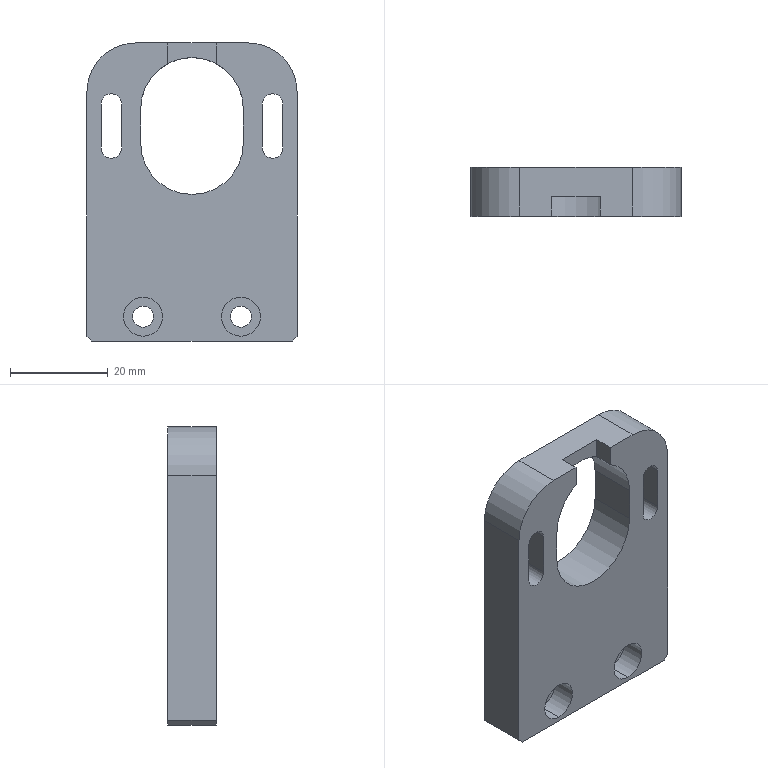Part | SolidWorks | features ICE 5, HoleWzd 2, MoveFace 2, Chamfer 1, Extrusion 1, Fillet 1 | 1 solid | 50 faces | box 43 x 10 x 61 mm | volume 18334 mm3 | cylinder 25 | plane 25 | commonest cylinder face diameters 8 x10 4.2 x6 4.3 x4 21 x3 20 x2
STEP:
#1=CARTESIAN_POINT('',(0.,4.,27.5));
#2=VERTEX_POINT('',#1);
#3=CARTESIAN_POINT('',(5.,4.,26.233));
#4=VERTEX_POINT('',#3);
#5=CARTESIAN_POINT('',(0.,4.,17.));
#6=DIRECTION('',(0.,1.,0.));
#7=DIRECTION('',(0.,0.,-1.));
#8=AXIS2_PLACEMENT_3D('',#5,#6,#7);
#9=CIRCLE('',#8,10.5);
#10=EDGE_CURVE('',#2,#4,#9,.T.);
#11=ORIENTED_EDGE('',*,*,#10,.F.);
#12=CARTESIAN_POINT('',(0.,10.,27.5));
#13=VERTEX_POINT('',#12);
#14=CARTESIAN_POINT('',(0.,0.,27.5));
#15=DIRECTION('',(0.,1.,0.));
#16=VECTOR('',#15,1000.);
#17=LINE('',#14,#16);
#18=EDGE_CURVE('',#2,#13,#17,.T.);
#19=ORIENTED_EDGE('',*,*,#18,.T.);
#20=CARTESIAN_POINT('',(10.5,10.,17.));
#21=VERTEX_POINT('',#20);
#22=CARTESIAN_POINT('',(0.,10.,17.));
#23=DIRECTION('',(0.,1.,0.));
#24=DIRECTION('',(0.,0.,1.));
#25=AXIS2_PLACEMENT_3D('',#22,#23,#24);
#26=CIRCLE('',#25,10.5);
#27=EDGE_CURVE('',#13,#21,#26,.T.);
#28=ORIENTED_EDGE('',*,*,#27,.T.);
#29=CARTESIAN_POINT('',(10.5,0.,17.));
#30=VERTEX_POINT('',#29);
#31=CARTESIAN_POINT('',(10.5,0.,17.));
#32=DIRECTION('',(0.,1.,0.));
#33=VECTOR('',#32,1000.);
#34=LINE('',#31,#33);
#35=EDGE_CURVE('',#30,#21,#34,.T.);
#36=ORIENTED_EDGE('',*,*,#35,.F.);
#37=CARTESIAN_POINT('',(5.,0.,26.233));
#38=VERTEX_POINT('',#37);
#39=CARTESIAN_POINT('',(0.,0.,17.));
#40=DIRECTION('',(0.,1.,0.));
#41=DIRECTION('',(0.,0.,1.));
#42=AXIS2_PLACEMENT_3D('',#39,#40,#41);
#43=CIRCLE('',#42,10.5);
#44=EDGE_CURVE('',#38,#30,#43,.T.);
#45=ORIENTED_EDGE('',*,*,#44,.F.);
#46=CARTESIAN_POINT('',(5.,0.,26.233));
#47=DIRECTION('',(0.,1.,0.));
#48=VECTOR('',#47,1000.);
#49=LINE('',#46,#48);
#50=EDGE_CURVE('',#38,#4,#49,.T.);
#51=ORIENTED_EDGE('',*,*,#50,.T.);
#52=EDGE_LOOP('',(#11,#19,#28,#36,#45,#51));
#53=FACE_OUTER_BOUND('',#52,.T.);
#54=CARTESIAN_POINT('',(0.,0.,17.));
#55=DIRECTION('',(0.,1.,0.));
#56=DIRECTION('',(0.,0.,1.));
#57=AXIS2_PLACEMENT_3D('',#54,#55,#56);
#58=CYLINDRICAL_SURFACE('',#57,10.5);
#59=ADVANCED_FACE('',(#53),#58,.F.);
#60=CARTESIAN_POINT('',(16.5,5.,22.));
#61=VERTEX_POINT('',#60);
#62=CARTESIAN_POINT('',(20.5,5.,18.));
#63=VERTEX_POINT('',#62);
#64=CARTESIAN_POINT('',(16.5,5.,18.));
#65=DIRECTION('',(0.,1.,0.));
#66=DIRECTION('',(0.,0.,1.));
#67=AXIS2_PLACEMENT_3D('',#64,#65,#66);
#68=CIRCLE('',#67,4.);
#69=EDGE_CURVE('',#61,#63,#68,.T.);
#70=ORIENTED_EDGE('',*,*,#69,.F.);
#71=CARTESIAN_POINT('',(16.5,10.,22.));
#72=VERTEX_POINT('',#71);
#73=CARTESIAN_POINT('',(16.5,5.,22.));
#74=DIRECTION('',(0.,1.,0.));
#75=VECTOR('',#74,1000.);
#76=LINE('',#73,#75);
#77=EDGE_CURVE('',#61,#72,#76,.T.);
#78=ORIENTED_EDGE('',*,*,#77,.T.);
#79=CARTESIAN_POINT('',(20.5,10.,18.));
#80=VERTEX_POINT('',#79);
#81=CARTESIAN_POINT('',(16.5,10.,18.));
#82=DIRECTION('',(0.,1.,0.));
#83=DIRECTION('',(0.,0.,1.));
#84=AXIS2_PLACEMENT_3D('',#81,#82,#83);
#85=CIRCLE('',#84,4.);
#86=EDGE_CURVE('',#72,#80,#85,.T.);
#87=ORIENTED_EDGE('',*,*,#86,.T.);
#88=CARTESIAN_POINT('',(20.5,5.,18.));
#89=DIRECTION('',(0.,1.,0.));
#90=VECTOR('',#89,1000.);
#91=LINE('',#88,#90);
#92=EDGE_CURVE('',#63,#80,#91,.T.);
#93=ORIENTED_EDGE('',*,*,#92,.F.);
#94=EDGE_LOOP('',(#70,#78,#87,#93));
#95=FACE_OUTER_BOUND('',#94,.T.);
#96=CARTESIAN_POINT('',(16.5,5.,18.));
#97=DIRECTION('',(0.,1.,0.));
#98=DIRECTION('',(0.,0.,1.));
#99=AXIS2_PLACEMENT_3D('',#96,#97,#98);
#100=CYLINDRICAL_SURFACE('',#99,4.);
#101=ADVANCED_FACE('',(#95),#100,.F.);
#102=CARTESIAN_POINT('',(-16.5,5.,22.));
#103=VERTEX_POINT('',#102);
#104=CARTESIAN_POINT('',(-12.5,5.,18.));
#105=VERTEX_POINT('',#104);
#106=CARTESIAN_POINT('',(-16.5,5.,18.));
#107=DIRECTION('',(0.,1.,0.));
#108=DIRECTION('',(0.,0.,1.));
#109=AXIS2_PLACEMENT_3D('',#106,#107,#108);
#110=CIRCLE('',#109,4.);
#111=EDGE_CURVE('',#103,#105,#110,.T.);
#112=ORIENTED_EDGE('',*,*,#111,.F.);
#113=CARTESIAN_POINT('',(-16.5,10.,22.));
#114=VERTEX_POINT('',#113);
#115=CARTESIAN_POINT('',(-16.5,5.,22.));
#116=DIRECTION('',(0.,1.,0.));
#117=VECTOR('',#116,1000.);
#118=LINE('',#115,#117);
#119=EDGE_CURVE('',#103,#114,#118,.T.);
#120=ORIENTED_EDGE('',*,*,#119,.T.);
#121=CARTESIAN_POINT('',(-12.5,10.,18.));
#122=VERTEX_POINT('',#121);
#123=CARTESIAN_POINT('',(-16.5,10.,18.));
#124=DIRECTION('',(0.,1.,0.));
#125=DIRECTION('',(0.,0.,1.));
#126=AXIS2_PLACEMENT_3D('',#123,#124,#125);
#127=CIRCLE('',#126,4.);
#128=EDGE_CURVE('',#114,#122,#127,.T.);
#129=ORIENTED_EDGE('',*,*,#128,.T.);
#130=CARTESIAN_POINT('',(-12.5,5.,18.));
#131=DIRECTION('',(0.,1.,0.));
#132=VECTOR('',#131,1000.);
#133=LINE('',#130,#132);
#134=EDGE_CURVE('',#105,#122,#133,.T.);
#135=ORIENTED_EDGE('',*,*,#134,.F.);
#136=EDGE_LOOP('',(#112,#120,#129,#135));
#137=FACE_OUTER_BOUND('',#136,.T.);
#138=CARTESIAN_POINT('',(-16.5,5.,18.));
#139=DIRECTION('',(0.,1.,0.));
#140=DIRECTION('',(0.,0.,1.));
#141=AXIS2_PLACEMENT_3D('',#138,#139,#140);
#142=CYLINDRICAL_SURFACE('',#141,4.);
#143=ADVANCED_FACE('',(#137),#142,.F.);
#144=CARTESIAN_POINT('',(-10.,5.,-21.5));
#145=VERTEX_POINT('',#144);
#146=CARTESIAN_POINT('',(-10.,5.,-29.5));
#147=VERTEX_POINT('',#146);
#148=CARTESIAN_POINT('',(-10.,5.,-25.5));
#149=DIRECTION('',(0.,-1.,0.));
#150=DIRECTION('',(0.,0.,-1.));
#151=AXIS2_PLACEMENT_3D('',#148,#149,#150);
#152=CIRCLE('',#151,4.);
#153=EDGE_CURVE('',#145,#147,#152,.T.);
#154=ORIENTED_EDGE('',*,*,#153,.F.);
#155=CARTESIAN_POINT('',(-10.,0.,-21.5));
#156=VERTEX_POINT('',#155);
#157=CARTESIAN_POINT('',(-10.,0.,-21.5));
#158=DIRECTION('',(0.,-1.,0.));
#159=VECTOR('',#158,1000.);
#160=LINE('',#157,#159);
#161=EDGE_CURVE('',#145,#156,#160,.T.);
#162=ORIENTED_EDGE('',*,*,#161,.T.);
#163=CARTESIAN_POINT('',(-10.,0.,-29.5));
#164=VERTEX_POINT('',#163);
#165=CARTESIAN_POINT('',(-10.,0.,-25.5));
#166=DIRECTION('',(0.,-1.,0.));
#167=DIRECTION('',(0.,0.,-1.));
#168=AXIS2_PLACEMENT_3D('',#165,#166,#167);
#169=CIRCLE('',#168,4.);
#170=EDGE_CURVE('',#156,#164,#169,.T.);
#171=ORIENTED_EDGE('',*,*,#170,.T.);
#172=CARTESIAN_POINT('',(-10.,0.,-29.5));
#173=DIRECTION('',(0.,-1.,0.));
#174=VECTOR('',#173,1000.);
#175=LINE('',#172,#174);
#176=EDGE_CURVE('',#147,#164,#175,.T.);
#177=ORIENTED_EDGE('',*,*,#176,.F.);
#178=EDGE_LOOP('',(#154,#162,#171,#177));
#179=FACE_OUTER_BOUND('',#178,.T.);
#180=CARTESIAN_POINT('',(-10.,0.,-25.5));
#181=DIRECTION('',(0.,-1.,0.));
#182=DIRECTION('',(0.,0.,-1.));
#183=AXIS2_PLACEMENT_3D('',#180,#181,#182);
#184=CYLINDRICAL_SURFACE('',#183,4.);
#185=ADVANCED_FACE('',(#179),#184,.F.);
#186=CARTESIAN_POINT('',(-10.,10.,-23.35));
#187=VERTEX_POINT('',#186);
#188=CARTESIAN_POINT('',(-10.,10.,-27.65));
#189=VERTEX_POINT('',#188);
#190=CARTESIAN_POINT('',(-10.,10.,-25.5));
#191=DIRECTION('',(0.,-1.,0.));
#192=DIRECTION('',(0.,0.,-1.));
#193=AXIS2_PLACEMENT_3D('',#190,#191,#192);
#194=CIRCLE('',#193,2.15);
#195=EDGE_CURVE('',#187,#189,#194,.T.);
#196=ORIENTED_EDGE('',*,*,#195,.F.);
#197=CARTESIAN_POINT('',(-10.,5.,-23.35));
#198=VERTEX_POINT('',#197);
#199=CARTESIAN_POINT('',(-10.,0.,-23.35));
#200=DIRECTION('',(0.,-1.,0.));
#201=VECTOR('',#200,1000.);
#202=LINE('',#199,#201);
#203=EDGE_CURVE('',#187,#198,#202,.T.);
#204=ORIENTED_EDGE('',*,*,#203,.T.);
#205=CARTESIAN_POINT('',(-10.,5.,-27.65));
#206=VERTEX_POINT('',#205);
#207=CARTESIAN_POINT('',(-10.,5.,-25.5));
#208=DIRECTION('',(0.,-1.,0.));
#209=DIRECTION('',(0.,0.,-1.));
#210=AXIS2_PLACEMENT_3D('',#207,#208,#209);
#211=CIRCLE('',#210,2.15);
#212=EDGE_CURVE('',#198,#206,#211,.T.);
#213=ORIENTED_EDGE('',*,*,#212,.T.);
#214=CARTESIAN_POINT('',(-10.,0.,-27.65));
#215=DIRECTION('',(0.,-1.,0.));
#216=VECTOR('',#215,1000.);
#217=LINE('',#214,#216);
#218=EDGE_CURVE('',#189,#206,#217,.T.);
#219=ORIENTED_EDGE('',*,*,#218,.F.);
#220=EDGE_LOOP('',(#196,#204,#213,#219));
#221=FACE_OUTER_BOUND('',#220,.T.);
#222=CARTESIAN_POINT('',(-10.,0.,-25.5));
#223=DIRECTION('',(0.,-1.,0.));
#224=DIRECTION('',(0.,0.,-1.));
#225=AXIS2_PLACEMENT_3D('',#222,#223,#224);
#226=CYLINDRICAL_SURFACE('',#225,2.15);
#227=ADVANCED_FACE('',(#221),#226,.F.);
#228=CARTESIAN_POINT('',(10.,5.,-21.5));
#229=VERTEX_POINT('',#228);
#230=CARTESIAN_POINT('',(10.,5.,-29.5));
#231=VERTEX_POINT('',#230);
#232=CARTESIAN_POINT('',(10.,5.,-25.5));
#233=DIRECTION('',(0.,-1.,0.));
#234=DIRECTION('',(0.,0.,-1.));
#235=AXIS2_PLACEMENT_3D('',#232,#233,#234);
#236=CIRCLE('',#235,4.);
#237=EDGE_CURVE('',#229,#231,#236,.T.);
#238=ORIENTED_EDGE('',*,*,#237,.F.);
#239=CARTESIAN_POINT('',(10.,0.,-21.5));
#240=VERTEX_POINT('',#239);
#241=CARTESIAN_POINT('',(10.,0.,-21.5));
#242=DIRECTION('',(0.,-1.,0.));
#243=VECTOR('',#242,1000.);
#244=LINE('',#241,#243);
#245=EDGE_CURVE('',#229,#240,#244,.T.);
#246=ORIENTED_EDGE('',*,*,#245,.T.);
#247=CARTESIAN_POINT('',(10.,0.,-29.5));
#248=VERTEX_POINT('',#247);
#249=CARTESIAN_POINT('',(10.,0.,-25.5));
#250=DIRECTION('',(0.,-1.,0.));
#251=DIRECTION('',(0.,0.,-1.));
#252=AXIS2_PLACEMENT_3D('',#249,#250,#251);
#253=CIRCLE('',#252,4.);
#254=EDGE_CURVE('',#240,#248,#253,.T.);
#255=ORIENTED_EDGE('',*,*,#254,.T.);
#256=CARTESIAN_POINT('',(10.,0.,-29.5));
#257=DIRECTION('',(0.,-1.,0.));
#258=VECTOR('',#257,1000.);
#259=LINE('',#256,#258);
#260=EDGE_CURVE('',#231,#248,#259,.T.);
#261=ORIENTED_EDGE('',*,*,#260,.F.);
#262=EDGE_LOOP('',(#238,#246,#255,#261));
#263=FACE_OUTER_BOUND('',#262,.T.);
#264=CARTESIAN_POINT('',(10.,0.,-25.5));
#265=DIRECTION('',(0.,-1.,0.));
#266=DIRECTION('',(0.,0.,-1.));
#267=AXIS2_PLACEMENT_3D('',#264,#265,#266);
#268=CYLINDRICAL_SURFACE('',#267,4.);
#269=ADVANCED_FACE('',(#263),#268,.F.);
#270=CARTESIAN_POINT('',(10.,10.,-23.35));
#271=VERTEX_POINT('',#270);
#272=CARTESIAN_POINT('',(10.,10.,-27.65));
#273=VERTEX_POINT('',#272);
#274=CARTESIAN_POINT('',(10.,10.,-25.5));
#275=DIRECTION('',(0.,-1.,0.));
#276=DIRECTION('',(0.,0.,-1.));
#277=AXIS2_PLACEMENT_3D('',#274,#275,#276);
#278=CIRCLE('',#277,2.15);
#279=EDGE_CURVE('',#271,#273,#278,.T.);
#280=ORIENTED_EDGE('',*,*,#279,.F.);
#281=CARTESIAN_POINT('',(10.,5.,-23.35));
#282=VERTEX_POINT('',#281);
#283=CARTESIAN_POINT('',(10.,0.,-23.35));
#284=DIRECTION('',(0.,-1.,0.));
#285=VECTOR('',#284,1000.);
#286=LINE('',#283,#285);
#287=EDGE_CURVE('',#271,#282,#286,.T.);
#288=ORIENTED_EDGE('',*,*,#287,.T.);
#289=CARTESIAN_POINT('',(10.,5.,-27.65));
#290=VERTEX_POINT('',#289);
#291=CARTESIAN_POINT('',(10.,5.,-25.5));
#292=DIRECTION('',(0.,-1.,0.));
#293=DIRECTION('',(0.,0.,-1.));
#294=AXIS2_PLACEMENT_3D('',#291,#292,#293);
#295=CIRCLE('',#294,2.15);
#296=EDGE_CURVE('',#282,#290,#295,.T.);
#297=ORIENTED_EDGE('',*,*,#296,.T.);
#298=CARTESIAN_POINT('',(10.,0.,-27.65));
#299=DIRECTION('',(0.,-1.,0.));
#300=VECTOR('',#299,1000.);
#301=LINE('',#298,#300);
#302=EDGE_CURVE('',#273,#290,#301,.T.);
#303=ORIENTED_EDGE('',*,*,#302,.F.);
#304=EDGE_LOOP('',(#280,#288,#297,#303));
#305=FACE_OUTER_BOUND('',#304,.T.);
#306=CARTESIAN_POINT('',(10.,0.,-25.5));
#307=DIRECTION('',(0.,-1.,0.));
#308=DIRECTION('',(0.,0.,-1.));
#309=AXIS2_PLACEMENT_3D('',#306,#307,#308);
#310=CYLINDRICAL_SURFACE('',#309,2.15);
#311=ADVANCED_FACE('',(#305),#310,.F.);
#312=CARTESIAN_POINT('',(-16.5,0.,20.1));
#313=VERTEX_POINT('',#312);
#314=CARTESIAN_POINT('',(-14.4,0.,18.));
#315=VERTEX_POINT('',#314);
#316=CARTESIAN_POINT('',(-16.5,0.,18.));
#317=DIRECTION('',(0.,1.,0.));
#318=DIRECTION('',(0.,0.,1.));
#319=AXIS2_PLACEMENT_3D('',#316,#317,#318);
#320=CIRCLE('',#319,2.1);
#321=EDGE_CURVE('',#313,#315,#320,.T.);
#322=ORIENTED_EDGE('',*,*,#321,.F.);
#323=CARTESIAN_POINT('',(-16.5,5.,20.1));
#324=VERTEX_POINT('',#323);
#325=CARTESIAN_POINT('',(-16.5,0.,20.1));
#326=DIRECTION('',(0.,1.,0.));
#327=VECTOR('',#326,1000.);
#328=LINE('',#325,#327);
#329=EDGE_CURVE('',#313,#324,#328,.T.);
#330=ORIENTED_EDGE('',*,*,#329,.T.);
#331=CARTESIAN_POINT('',(-14.4,5.,18.));
#332=VERTEX_POINT('',#331);
#333=CARTESIAN_POINT('',(-16.5,5.,18.));
#334=DIRECTION('',(0.,-1.,0.));
#335=DIRECTION('',(0.,0.,-1.));
#336=AXIS2_PLACEMENT_3D('',#333,#334,#335);
#337=CIRCLE('',#336,2.1);
#338=EDGE_CURVE('',#332,#324,#337,.T.);
#339=ORIENTED_EDGE('',*,*,#338,.F.);
#340=CARTESIAN_POINT('',(-14.4,0.,18.));
#341=DIRECTION('',(0.,1.,0.));
#342=VECTOR('',#341,1000.);
#343=LINE('',#340,#342);
#344=EDGE_CURVE('',#315,#332,#343,.T.);
#345=ORIENTED_EDGE('',*,*,#344,.F.);
#346=EDGE_LOOP('',(#322,#330,#339,#345));
#347=FACE_OUTER_BOUND('',#346,.T.);
#348=CARTESIAN_POINT('',(-16.5,0.,18.));
#349=DIRECTION('',(0.,1.,0.));
#350=DIRECTION('',(0.,0.,1.));
#351=AXIS2_PLACEMENT_3D('',#348,#349,#350);
#352=CYLINDRICAL_SURFACE('',#351,2.1);
#353=ADVANCED_FACE('',(#347),#352,.F.);
#354=CARTESIAN_POINT('',(16.5,0.,20.1));
#355=VERTEX_POINT('',#354);
#356=CARTESIAN_POINT('',(18.6,0.,18.));
#357=VERTEX_POINT('',#356);
#358=CARTESIAN_POINT('',(16.5,0.,18.));
#359=DIRECTION('',(0.,1.,0.));
#360=DIRECTION('',(0.,0.,1.));
#361=AXIS2_PLACEMENT_3D('',#358,#359,#360);
#362=CIRCLE('',#361,2.1);
#363=EDGE_CURVE('',#355,#357,#362,.T.);
#364=ORIENTED_EDGE('',*,*,#363,.F.);
#365=CARTESIAN_POINT('',(16.5,5.,20.1));
#366=VERTEX_POINT('',#365);
#367=CARTESIAN_POINT('',(16.5,0.,20.1));
#368=DIRECTION('',(0.,1.,0.));
#369=VECTOR('',#368,1000.);
#370=LINE('',#367,#369);
#371=EDGE_CURVE('',#355,#366,#370,.T.);
#372=ORIENTED_EDGE('',*,*,#371,.T.);
#373=CARTESIAN_POINT('',(18.6,5.,18.));
#374=VERTEX_POINT('',#373);
#375=CARTESIAN_POINT('',(16.5,5.,18.));
#376=DIRECTION('',(0.,-1.,0.));
#377=DIRECTION('',(0.,0.,-1.));
#378=AXIS2_PLACEMENT_3D('',#375,#376,#377);
#379=CIRCLE('',#378,2.1);
#380=EDGE_CURVE('',#374,#366,#379,.T.);
#381=ORIENTED_EDGE('',*,*,#380,.F.);
#382=CARTESIAN_POINT('',(18.6,0.,18.));
#383=DIRECTION('',(0.,1.,0.));
#384=VECTOR('',#383,1000.);
#385=LINE('',#382,#384);
#386=EDGE_CURVE('',#357,#374,#385,.T.);
#387=ORIENTED_EDGE('',*,*,#386,.F.);
#388=EDGE_LOOP('',(#364,#372,#381,#387));
#389=FACE_OUTER_BOUND('',#388,.T.);
#390=CARTESIAN_POINT('',(16.5,0.,18.));
#391=DIRECTION('',(0.,1.,0.));
#392=DIRECTION('',(0.,0.,1.));
#393=AXIS2_PLACEMENT_3D('',#390,#391,#392);
#394=CYLINDRICAL_SURFACE('',#393,2.1);
#395=ADVANCED_FACE('',(#389),#394,.F.);
#396=CARTESIAN_POINT('',(18.6,5.,9.));
#397=VERTEX_POINT('',#396);
#398=CARTESIAN_POINT('',(18.6,5.,17.5));
#399=DIRECTION('',(0.,0.,1.));
#400=VECTOR('',#399,1000.);
#401=LINE('',#398,#400);
#402=EDGE_CURVE('',#397,#374,#401,.T.);
#403=ORIENTED_EDGE('',*,*,#402,.F.);
#404=CARTESIAN_POINT('',(18.6,0.,9.));
#405=VERTEX_POINT('',#404);
#406=CARTESIAN_POINT('',(18.6,0.,9.));
#407=DIRECTION('',(0.,1.,0.));
#408=VECTOR('',#407,1000.);
#409=LINE('',#406,#408);
#410=EDGE_CURVE('',#405,#397,#409,.T.);
#411=ORIENTED_EDGE('',*,*,#410,.F.);
#412=CARTESIAN_POINT('',(18.6,0.,11.));
#413=DIRECTION('',(0.,0.,-1.));
#414=VECTOR('',#413,1000.);
#415=LINE('',#412,#414);
#416=EDGE_CURVE('',#357,#405,#415,.T.);
#417=ORIENTED_EDGE('',*,*,#416,.F.);
#418=ORIENTED_EDGE('',*,*,#386,.T.);
#419=EDGE_LOOP('',(#403,#411,#417,#418));
#420=FACE_OUTER_BOUND('',#419,.T.);
#421=CARTESIAN_POINT('',(18.6,0.,11.));
#422=DIRECTION('',(1.,0.,0.));
#423=DIRECTION('',(0.,0.,-1.));
#424=AXIS2_PLACEMENT_3D('',#421,#422,#423);
#425=PLANE('',#424);
#426=ADVANCED_FACE('',(#420),#425,.F.);
#427=ORIENTED_EDGE('',*,*,#371,.F.);
#428=CARTESIAN_POINT('',(14.4,0.,18.));
#429=VERTEX_POINT('',#428);
#430=CARTESIAN_POINT('',(16.5,0.,18.));
#431=DIRECTION('',(0.,1.,0.));
#432=DIRECTION('',(0.,0.,1.));
#433=AXIS2_PLACEMENT_3D('',#430,#431,#432);
#434=CIRCLE('',#433,2.1);
#435=EDGE_CURVE('',#429,#355,#434,.T.);
#436=ORIENTED_EDGE('',*,*,#435,.F.);
#437=CARTESIAN_POINT('',(14.4,5.,18.));
#438=VERTEX_POINT('',#437);
#439=CARTESIAN_POINT('',(14.4,0.,18.));
#440=DIRECTION('',(0.,1.,0.));
#441=VECTOR('',#440,1000.);
#442=LINE('',#439,#441);
#443=EDGE_CURVE('',#429,#438,#442,.T.);
#444=ORIENTED_EDGE('',*,*,#443,.T.);
#445=CARTESIAN_POINT('',(16.5,5.,18.));
#446=DIRECTION('',(0.,-1.,0.));
#447=DIRECTION('',(0.,0.,-1.));
#448=AXIS2_PLACEMENT_3D('',#445,#446,#447);
#449=CIRCLE('',#448,2.1);
#450=EDGE_CURVE('',#366,#438,#449,.T.);
#451=ORIENTED_EDGE('',*,*,#450,.F.);
#452=EDGE_LOOP('',(#427,#436,#444,#451));
#453=FACE_OUTER_BOUND('',#452,.T.);
#454=CARTESIAN_POINT('',(16.5,0.,18.));
#455=DIRECTION('',(0.,1.,0.));
#456=DIRECTION('',(0.,0.,1.));
#457=AXIS2_PLACEMENT_3D('',#454,#455,#456);
#458=CYLINDRICAL_SURFACE('',#457,2.1);
#459=ADVANCED_FACE('',(#453),#458,.F.);
#460=CARTESIAN_POINT('',(14.4,0.,9.));
#461=VERTEX_POINT('',#460);
#462=CARTESIAN_POINT('',(14.4,5.,9.));
#463=VERTEX_POINT('',#462);
#464=CARTESIAN_POINT('',(14.4,0.,9.));
#465=DIRECTION('',(0.,1.,0.));
#466=VECTOR('',#465,1000.);
#467=LINE('',#464,#466);
#468=EDGE_CURVE('',#461,#463,#467,.T.);
#469=ORIENTED_EDGE('',*,*,#468,.T.);
#470=CARTESIAN_POINT('',(14.4,5.,17.5));
#471=DIRECTION('',(0.,0.,-1.));
#472=VECTOR('',#471,1000.);
#473=LINE('',#470,#472);
#474=EDGE_CURVE('',#438,#463,#473,.T.);
#475=ORIENTED_EDGE('',*,*,#474,.F.);
#476=ORIENTED_EDGE('',*,*,#443,.F.);
#477=CARTESIAN_POINT('',(14.4,0.,11.));
#478=DIRECTION('',(0.,0.,1.));
#479=VECTOR('',#478,1000.);
#480=LINE('',#477,#479);
#481=EDGE_CURVE('',#461,#429,#480,.T.);
#482=ORIENTED_EDGE('',*,*,#481,.F.);
#483=EDGE_LOOP('',(#469,#475,#476,#482));
#484=FACE_OUTER_BOUND('',#483,.T.);
#485=CARTESIAN_POINT('',(14.4,0.,11.));
#486=DIRECTION('',(-1.,0.,0.));
#487=DIRECTION('',(0.,0.,1.));
#488=AXIS2_PLACEMENT_3D('',#485,#486,#487);
#489=PLANE('',#488);
#490=ADVANCED_FACE('',(#484),#489,.F.);
#491=CARTESIAN_POINT('',(16.5,5.,9.));
#492=DIRECTION('',(0.,-1.,0.));
#493=DIRECTION('',(0.,0.,1.));
#494=AXIS2_PLACEMENT_3D('',#491,#492,#493);
#495=CIRCLE('',#494,2.1);
#496=EDGE_CURVE('',#463,#397,#495,.T.);
#497=ORIENTED_EDGE('',*,*,#496,.F.);
#498=ORIENTED_EDGE('',*,*,#468,.F.);
#499=CARTESIAN_POINT('',(16.5,0.,9.));
#500=DIRECTION('',(0.,1.,0.));
#501=DIRECTION('',(0.,0.,1.));
#502=AXIS2_PLACEMENT_3D('',#499,#500,#501);
#503=CIRCLE('',#502,2.1);
#504=EDGE_CURVE('',#405,#461,#503,.T.);
#505=ORIENTED_EDGE('',*,*,#504,.F.);
#506=ORIENTED_EDGE('',*,*,#410,.T.);
#507=EDGE_LOOP('',(#497,#498,#505,#506));
#508=FACE_OUTER_BOUND('',#507,.T.);
#509=CARTESIAN_POINT('',(16.5,0.,9.));
#510=DIRECTION('',(0.,1.,0.));
#511=DIRECTION('',(0.,0.,1.));
#512=AXIS2_PLACEMENT_3D('',#509,#510,#511);
#513=CYLINDRICAL_SURFACE('',#512,2.1);
#514=ADVANCED_FACE('',(#508),#513,.F.);
#515=CARTESIAN_POINT('',(-14.4,5.,9.));
#516=VERTEX_POINT('',#515);
#517=CARTESIAN_POINT('',(-14.4,5.,17.5));
#518=DIRECTION('',(0.,0.,1.));
#519=VECTOR('',#518,1000.);
#520=LINE('',#517,#519);
#521=EDGE_CURVE('',#516,#332,#520,.T.);
#522=ORIENTED_EDGE('',*,*,#521,.F.);
#523=CARTESIAN_POINT('',(-14.4,0.,9.));
#524=VERTEX_POINT('',#523);
#525=CARTESIAN_POINT('',(-14.4,0.,9.));
#526=DIRECTION('',(0.,1.,0.));
#527=VECTOR('',#526,1000.);
#528=LINE('',#525,#527);
#529=EDGE_CURVE('',#524,#516,#528,.T.);
#530=ORIENTED_EDGE('',*,*,#529,.F.);
#531=CARTESIAN_POINT('',(-14.4,0.,11.));
#532=DIRECTION('',(0.,0.,-1.));
#533=VECTOR('',#532,1000.);
#534=LINE('',#531,#533);
#535=EDGE_CURVE('',#315,#524,#534,.T.);
#536=ORIENTED_EDGE('',*,*,#535,.F.);
#537=ORIENTED_EDGE('',*,*,#344,.T.);
#538=EDGE_LOOP('',(#522,#530,#536,#537));
#539=FACE_OUTER_BOUND('',#538,.T.);
#540=CARTESIAN_POINT('',(-14.4,0.,11.));
#541=DIRECTION('',(1.,0.,0.));
#542=DIRECTION('',(0.,0.,-1.));
#543=AXIS2_PLACEMENT_3D('',#540,#541,#542);
#544=PLANE('',#543);
#545=ADVANCED_FACE('',(#539),#544,.F.);
#546=ORIENTED_EDGE('',*,*,#329,.F.);
#547=CARTESIAN_POINT('',(-18.6,0.,18.));
#548=VERTEX_POINT('',#547);
#549=CARTESIAN_POINT('',(-16.5,0.,18.));
#550=DIRECTION('',(0.,1.,0.));
#551=DIRECTION('',(0.,0.,1.));
#552=AXIS2_PLACEMENT_3D('',#549,#550,#551);
#553=CIRCLE('',#552,2.1);
#554=EDGE_CURVE('',#548,#313,#553,.T.);
#555=ORIENTED_EDGE('',*,*,#554,.F.);
#556=CARTESIAN_POINT('',(-18.6,5.,18.));
#557=VERTEX_POINT('',#556);
#558=CARTESIAN_POINT('',(-18.6,0.,18.));
#559=DIRECTION('',(0.,1.,0.));
#560=VECTOR('',#559,1000.);
#561=LINE('',#558,#560);
#562=EDGE_CURVE('',#548,#557,#561,.T.);
#563=ORIENTED_EDGE('',*,*,#562,.T.);
#564=CARTESIAN_POINT('',(-16.5,5.,18.));
#565=DIRECTION('',(0.,-1.,0.));
#566=DIRECTION('',(0.,0.,-1.));
#567=AXIS2_PLACEMENT_3D('',#564,#565,#566);
#568=CIRCLE('',#567,2.1);
#569=EDGE_CURVE('',#324,#557,#568,.T.);
#570=ORIENTED_EDGE('',*,*,#569,.F.);
#571=EDGE_LOOP('',(#546,#555,#563,#570));
#572=FACE_OUTER_BOUND('',#571,.T.);
#573=CARTESIAN_POINT('',(-16.5,0.,18.));
#574=DIRECTION('',(0.,1.,0.));
#575=DIRECTION('',(0.,0.,1.));
#576=AXIS2_PLACEMENT_3D('',#573,#574,#575);
#577=CYLINDRICAL_SURFACE('',#576,2.1);
#578=ADVANCED_FACE('',(#572),#577,.F.);
#579=CARTESIAN_POINT('',(-18.6,0.,9.));
#580=VERTEX_POINT('',#579);
#581=CARTESIAN_POINT('',(-18.6,5.,9.));
#582=VERTEX_POINT('',#581);
#583=CARTESIAN_POINT('',(-18.6,0.,9.));
#584=DIRECTION('',(0.,1.,0.));
#585=VECTOR('',#584,1000.);
#586=LINE('',#583,#585);
#587=EDGE_CURVE('',#580,#582,#586,.T.);
#588=ORIENTED_EDGE('',*,*,#587,.T.);
#589=CARTESIAN_POINT('',(-18.6,5.,17.5));
#590=DIRECTION('',(0.,0.,-1.));
#591=VECTOR('',#590,1000.);
#592=LINE('',#589,#591);
#593=EDGE_CURVE('',#557,#582,#592,.T.);
#594=ORIENTED_EDGE('',*,*,#593,.F.);
#595=ORIENTED_EDGE('',*,*,#562,.F.);
#596=CARTESIAN_POINT('',(-18.6,0.,11.));
#597=DIRECTION('',(0.,0.,1.));
#598=VECTOR('',#597,1000.);
#599=LINE('',#596,#598);
#600=EDGE_CURVE('',#580,#548,#599,.T.);
#601=ORIENTED_EDGE('',*,*,#600,.F.);
#602=EDGE_LOOP('',(#588,#594,#595,#601));
#603=FACE_OUTER_BOUND('',#602,.T.);
#604=CARTESIAN_POINT('',(-18.6,0.,11.));
#605=DIRECTION('',(-1.,0.,0.));
#606=DIRECTION('',(0.,0.,1.));
#607=AXIS2_PLACEMENT_3D('',#604,#605,#606);
#608=PLANE('',#607);
#609=ADVANCED_FACE('',(#603),#608,.F.);
#610=CARTESIAN_POINT('',(-16.5,5.,9.));
#611=DIRECTION('',(0.,-1.,0.));
#612=DIRECTION('',(0.,0.,1.));
#613=AXIS2_PLACEMENT_3D('',#610,#611,#612);
#614=CIRCLE('',#613,2.1);
#615=EDGE_CURVE('',#582,#516,#614,.T.);
#616=ORIENTED_EDGE('',*,*,#615,.F.);
#617=ORIENTED_EDGE('',*,*,#587,.F.);
#618=CARTESIAN_POINT('',(-16.5,0.,9.));
#619=DIRECTION('',(0.,1.,0.));
#620=DIRECTION('',(0.,0.,1.));
#621=AXIS2_PLACEMENT_3D('',#618,#619,#620);
#622=CIRCLE('',#621,2.1);
#623=EDGE_CURVE('',#524,#580,#622,.T.);
#624=ORIENTED_EDGE('',*,*,#623,.F.);
#625=ORIENTED_EDGE('',*,*,#529,.T.);
#626=EDGE_LOOP('',(#616,#617,#624,#625));
#627=FACE_OUTER_BOUND('',#626,.T.);
#628=CARTESIAN_POINT('',(-16.5,0.,9.));
#629=DIRECTION('',(0.,1.,0.));
#630=DIRECTION('',(0.,0.,1.));
#631=AXIS2_PLACEMENT_3D('',#628,#629,#630);
#632=CYLINDRICAL_SURFACE('',#631,2.1);
#633=ADVANCED_FACE('',(#627),#632,.F.);
#634=CARTESIAN_POINT('',(21.5,10.,20.5));
#635=VERTEX_POINT('',#634);
#636=CARTESIAN_POINT('',(21.5,10.,-29.5));
#637=VERTEX_POINT('',#636);
#638=CARTESIAN_POINT('',(21.5,10.,-32.5));
#639=DIRECTION('',(0.,0.,-1.));
#640=VECTOR('',#639,1000.);
#641=LINE('',#638,#640);
#642=EDGE_CURVE('',#635,#637,#641,.T.);
#643=ORIENTED_EDGE('',*,*,#642,.F.);
#644=CARTESIAN_POINT('',(21.5,0.,20.5));
#645=VERTEX_POINT('',#644);
#646=CARTESIAN_POINT('',(21.5,10.,20.5));
#647=DIRECTION('',(0.,-1.,0.));
#648=VECTOR('',#647,1000.);
#649=LINE('',#646,#648);
#650=EDGE_CURVE('',#635,#645,#649,.T.);
#651=ORIENTED_EDGE('',*,*,#650,.T.);
#652=CARTESIAN_POINT('',(21.5,0.,-29.5));
#653=VERTEX_POINT('',#652);
#654=CARTESIAN_POINT('',(21.5,0.,-32.5));
#655=DIRECTION('',(0.,0.,-1.));
#656=VECTOR('',#655,1000.);
#657=LINE('',#654,#656);
#658=EDGE_CURVE('',#645,#653,#657,.T.);
#659=ORIENTED_EDGE('',*,*,#658,.T.);
#660=CARTESIAN_POINT('',(21.5,10.,-29.5));
#661=DIRECTION('',(0.,1.,0.));
#662=VECTOR('',#661,1000.);
#663=LINE('',#660,#662);
#664=EDGE_CURVE('',#653,#637,#663,.T.);
#665=ORIENTED_EDGE('',*,*,#664,.T.);
#666=EDGE_LOOP('',(#643,#651,#659,#665));
#667=FACE_OUTER_BOUND('',#666,.T.);
#668=CARTESIAN_POINT('',(21.5,10.,-32.5));
#669=DIRECTION('',(-1.,0.,0.));
#670=DIRECTION('',(0.,0.,1.));
#671=AXIS2_PLACEMENT_3D('',#668,#669,#670);
#672=PLANE('',#671);
#673=ADVANCED_FACE('',(#667),#672,.F.);
#674=CARTESIAN_POINT('',(20.5,0.,-30.5));
#675=VERTEX_POINT('',#674);
#676=CARTESIAN_POINT('',(-20.5,0.,-30.5));
#677=VERTEX_POINT('',#676);
#678=CARTESIAN_POINT('',(-21.5,0.,-30.5));
#679=DIRECTION('',(-1.,0.,0.));
#680=VECTOR('',#679,1000.);
#681=LINE('',#678,#680);
#682=EDGE_CURVE('',#675,#677,#681,.T.);
#683=ORIENTED_EDGE('',*,*,#682,.T.);
#684=CARTESIAN_POINT('',(-20.5,10.,-30.5));
#685=VERTEX_POINT('',#684);
#686=CARTESIAN_POINT('',(-20.5,10.,-30.5));
#687=DIRECTION('',(0.,1.,0.));
#688=VECTOR('',#687,1000.);
#689=LINE('',#686,#688);
#690=EDGE_CURVE('',#677,#685,#689,.T.);
#691=ORIENTED_EDGE('',*,*,#690,.T.);
#692=CARTESIAN_POINT('',(20.5,10.,-30.5));
#693=VERTEX_POINT('',#692);
#694=CARTESIAN_POINT('',(-21.5,10.,-30.5));
#695=DIRECTION('',(-1.,0.,0.));
#696=VECTOR('',#695,1000.);
#697=LINE('',#694,#696);
#698=EDGE_CURVE('',#693,#685,#697,.T.);
#699=ORIENTED_EDGE('',*,*,#698,.F.);
#700=CARTESIAN_POINT('',(20.5,10.,-30.5));
#701=DIRECTION('',(0.,-1.,0.));
#702=VECTOR('',#701,1000.);
#703=LINE('',#700,#702);
#704=EDGE_CURVE('',#693,#675,#703,.T.);
#705=ORIENTED_EDGE('',*,*,#704,.T.);
#706=EDGE_LOOP('',(#683,#691,#699,#705));
#707=FACE_OUTER_BOUND('',#706,.T.);
#708=CARTESIAN_POINT('',(-21.5,10.,-30.5));
#709=DIRECTION('',(0.,0.,1.));
#710=DIRECTION('',(1.,0.,0.));
#711=AXIS2_PLACEMENT_3D('',#708,#709,#710);
#712=PLANE('',#711);
#713=ADVANCED_FACE('',(#707),#712,.F.);
#714=CARTESIAN_POINT('',(-21.5,0.,-29.5));
#715=VERTEX_POINT('',#714);
#716=CARTESIAN_POINT('',(-21.5,0.,20.5));
#717=VERTEX_POINT('',#716);
#718=CARTESIAN_POINT('',(-21.5,0.,-32.5));
#719=DIRECTION('',(0.,0.,1.));
#720=VECTOR('',#719,1000.);
#721=LINE('',#718,#720);
#722=EDGE_CURVE('',#715,#717,#721,.T.);
#723=ORIENTED_EDGE('',*,*,#722,.T.);
#724=CARTESIAN_POINT('',(-21.5,10.,20.5));
#725=VERTEX_POINT('',#724);
#726=CARTESIAN_POINT('',(-21.5,10.,20.5));
#727=DIRECTION('',(0.,1.,0.));
#728=VECTOR('',#727,1000.);
#729=LINE('',#726,#728);
#730=EDGE_CURVE('',#717,#725,#729,.T.);
#731=ORIENTED_EDGE('',*,*,#730,.T.);
#732=CARTESIAN_POINT('',(-21.5,10.,-29.5));
#733=VERTEX_POINT('',#732);
#734=CARTESIAN_POINT('',(-21.5,10.,-32.5));
#735=DIRECTION('',(0.,0.,1.));
#736=VECTOR('',#735,1000.);
#737=LINE('',#734,#736);
#738=EDGE_CURVE('',#733,#725,#737,.T.);
#739=ORIENTED_EDGE('',*,*,#738,.F.);
#740=CARTESIAN_POINT('',(-21.5,10.,-29.5));
#741=DIRECTION('',(0.,-1.,0.));
#742=VECTOR('',#741,1000.);
#743=LINE('',#740,#742);
#744=EDGE_CURVE('',#733,#715,#743,.T.);
#745=ORIENTED_EDGE('',*,*,#744,.T.);
#746=EDGE_LOOP('',(#723,#731,#739,#745));
#747=FACE_OUTER_BOUND('',#746,.T.);
#748=CARTESIAN_POINT('',(-21.5,10.,-32.5));
#749=DIRECTION('',(1.,0.,0.));
#750=DIRECTION('',(0.,0.,-1.));
#751=AXIS2_PLACEMENT_3D('',#748,#749,#750);
#752=PLANE('',#751);
#753=ADVANCED_FACE('',(#747),#752,.F.);
#754=CARTESIAN_POINT('',(5.,4.,30.5));
#755=VERTEX_POINT('',#754);
#756=CARTESIAN_POINT('',(-5.,4.,30.5));
#757=VERTEX_POINT('',#756);
#758=CARTESIAN_POINT('',(-21.5,4.,30.5));
#759=DIRECTION('',(-1.,0.,0.));
#760=VECTOR('',#759,1000.);
#761=LINE('',#758,#760);
#762=EDGE_CURVE('',#755,#757,#761,.T.);
#763=ORIENTED_EDGE('',*,*,#762,.F.);
#764=CARTESIAN_POINT('',(5.,0.,30.5));
#765=VERTEX_POINT('',#764);
#766=CARTESIAN_POINT('',(5.,10.,30.5));
#767=DIRECTION('',(0.,-1.,0.));
#768=VECTOR('',#767,1000.);
#769=LINE('',#766,#768);
#770=EDGE_CURVE('',#755,#765,#769,.T.);
#771=ORIENTED_EDGE('',*,*,#770,.T.);
#772=CARTESIAN_POINT('',(11.5,0.,30.5));
#773=VERTEX_POINT('',#772);
#774=CARTESIAN_POINT('',(-21.5,0.,30.5));
#775=DIRECTION('',(1.,0.,0.));
#776=VECTOR('',#775,1000.);
#777=LINE('',#774,#776);
#778=EDGE_CURVE('',#765,#773,#777,.T.);
#779=ORIENTED_EDGE('',*,*,#778,.T.);
#780=CARTESIAN_POINT('',(11.5,10.,30.5));
#781=VERTEX_POINT('',#780);
#782=CARTESIAN_POINT('',(11.5,10.,30.5));
#783=DIRECTION('',(0.,1.,0.));
#784=VECTOR('',#783,1000.);
#785=LINE('',#782,#784);
#786=EDGE_CURVE('',#773,#781,#785,.T.);
#787=ORIENTED_EDGE('',*,*,#786,.T.);
#788=CARTESIAN_POINT('',(-11.5,10.,30.5));
#789=VERTEX_POINT('',#788);
#790=CARTESIAN_POINT('',(-21.5,10.,30.5));
#791=DIRECTION('',(1.,0.,0.));
#792=VECTOR('',#791,1000.);
#793=LINE('',#790,#792);
#794=EDGE_CURVE('',#789,#781,#793,.T.);
#795=ORIENTED_EDGE('',*,*,#794,.F.);
#796=CARTESIAN_POINT('',(-11.5,0.,30.5));
#797=VERTEX_POINT('',#796);
#798=CARTESIAN_POINT('',(-11.5,10.,30.5));
#799=DIRECTION('',(0.,-1.,0.));
#800=VECTOR('',#799,1000.);
#801=LINE('',#798,#800);
#802=EDGE_CURVE('',#789,#797,#801,.T.);
#803=ORIENTED_EDGE('',*,*,#802,.T.);
#804=CARTESIAN_POINT('',(-5.,0.,30.5));
#805=VERTEX_POINT('',#804);
#806=CARTESIAN_POINT('',(-21.5,0.,30.5));
#807=DIRECTION('',(1.,0.,0.));
#808=VECTOR('',#807,1000.);
#809=LINE('',#806,#808);
#810=EDGE_CURVE('',#797,#805,#809,.T.);
#811=ORIENTED_EDGE('',*,*,#810,.T.);
#812=CARTESIAN_POINT('',(-5.,10.,30.5));
#813=DIRECTION('',(0.,1.,0.));
#814=VECTOR('',#813,1000.);
#815=LINE('',#812,#814);
#816=EDGE_CURVE('',#805,#757,#815,.T.);
#817=ORIENTED_EDGE('',*,*,#816,.T.);
#818=EDGE_LOOP('',(#763,#771,#779,#787,#795,#803,#811,#817));
#819=FACE_OUTER_BOUND('',#818,.T.);
#820=CARTESIAN_POINT('',(-21.5,10.,30.5));
#821=DIRECTION('',(0.,0.,-1.));
#822=DIRECTION('',(-1.,0.,0.));
#823=AXIS2_PLACEMENT_3D('',#820,#821,#822);
#824=PLANE('',#823);
#825=ADVANCED_FACE('',(#819),#824,.F.);
#826=CARTESIAN_POINT('',(10.5,10.,10.));
#827=VERTEX_POINT('',#826);
#828=CARTESIAN_POINT('',(10.5,10.,12.));
#829=DIRECTION('',(0.,0.,-1.));
#830=VECTOR('',#829,1000.);
#831=LINE('',#828,#830);
#832=EDGE_CURVE('',#21,#827,#831,.T.);
#833=ORIENTED_EDGE('',*,*,#832,.F.);
#834=ORIENTED_EDGE('',*,*,#27,.F.);
#835=CARTESIAN_POINT('',(-10.5,10.,17.));
#836=VERTEX_POINT('',#835);
#837=CARTESIAN_POINT('',(0.,10.,17.));
#838=DIRECTION('',(0.,1.,0.));
#839=DIRECTION('',(0.,0.,1.));
#840=AXIS2_PLACEMENT_3D('',#837,#838,#839);
#841=CIRCLE('',#840,10.5);
#842=EDGE_CURVE('',#836,#13,#841,.T.);
#843=ORIENTED_EDGE('',*,*,#842,.F.);
#844=CARTESIAN_POINT('',(-10.5,10.,10.));
#845=VERTEX_POINT('',#844);
#846=CARTESIAN_POINT('',(-10.5,10.,12.));
#847=DIRECTION('',(0.,0.,1.));
#848=VECTOR('',#847,1000.);
#849=LINE('',#846,#848);
#850=EDGE_CURVE('',#845,#836,#849,.T.);
#851=ORIENTED_EDGE('',*,*,#850,.F.);
#852=CARTESIAN_POINT('',(0.,10.,10.));
#853=DIRECTION('',(0.,1.,0.));
#854=DIRECTION('',(0.,0.,1.));
#855=AXIS2_PLACEMENT_3D('',#852,#853,#854);
#856=CIRCLE('',#855,10.5);
#857=EDGE_CURVE('',#827,#845,#856,.T.);
#858=ORIENTED_EDGE('',*,*,#857,.F.);
#859=EDGE_LOOP('',(#833,#834,#843,#851,#858));
#860=FACE_BOUND('',#859,.T.);
#861=CARTESIAN_POINT('',(20.5,10.,9.));
#862=VERTEX_POINT('',#861);
#863=CARTESIAN_POINT('',(12.5,10.,9.));
#864=VERTEX_POINT('',#863);
#865=CARTESIAN_POINT('',(16.5,10.,9.));
#866=DIRECTION('',(0.,1.,0.));
#867=DIRECTION('',(0.,0.,1.));
#868=AXIS2_PLACEMENT_3D('',#865,#866,#867);
#869=CIRCLE('',#868,4.);
#870=EDGE_CURVE('',#862,#864,#869,.T.);
#871=ORIENTED_EDGE('',*,*,#870,.F.);
#872=CARTESIAN_POINT('',(20.5,10.,11.));
#873=DIRECTION('',(0.,0.,-1.));
#874=VECTOR('',#873,1000.);
#875=LINE('',#872,#874);
#876=EDGE_CURVE('',#80,#862,#875,.T.);
#877=ORIENTED_EDGE('',*,*,#876,.F.);
#878=ORIENTED_EDGE('',*,*,#86,.F.);
#879=CARTESIAN_POINT('',(12.5,10.,18.));
#880=VERTEX_POINT('',#879);
#881=CARTESIAN_POINT('',(16.5,10.,18.));
#882=DIRECTION('',(0.,1.,0.));
#883=DIRECTION('',(0.,0.,1.));
#884=AXIS2_PLACEMENT_3D('',#881,#882,#883);
#885=CIRCLE('',#884,4.);
#886=EDGE_CURVE('',#880,#72,#885,.T.);
#887=ORIENTED_EDGE('',*,*,#886,.F.);
#888=CARTESIAN_POINT('',(12.5,10.,11.));
#889=DIRECTION('',(0.,0.,1.));
#890=VECTOR('',#889,1000.);
#891=LINE('',#888,#890);
#892=EDGE_CURVE('',#864,#880,#891,.T.);
#893=ORIENTED_EDGE('',*,*,#892,.F.);
#894=EDGE_LOOP('',(#871,#877,#878,#887,#893));
#895=FACE_BOUND('',#894,.T.);
#896=CARTESIAN_POINT('',(-12.5,10.,9.));
#897=VERTEX_POINT('',#896);
#898=CARTESIAN_POINT('',(-20.5,10.,9.));
#899=VERTEX_POINT('',#898);
#900=CARTESIAN_POINT('',(-16.5,10.,9.));
#901=DIRECTION('',(0.,1.,0.));
#902=DIRECTION('',(0.,0.,1.));
#903=AXIS2_PLACEMENT_3D('',#900,#901,#902);
#904=CIRCLE('',#903,4.);
#905=EDGE_CURVE('',#897,#899,#904,.T.);
#906=ORIENTED_EDGE('',*,*,#905,.F.);
#907=CARTESIAN_POINT('',(-12.5,10.,11.));
#908=DIRECTION('',(0.,0.,-1.));
#909=VECTOR('',#908,1000.);
#910=LINE('',#907,#909);
#911=EDGE_CURVE('',#122,#897,#910,.T.);
#912=ORIENTED_EDGE('',*,*,#911,.F.);
#913=ORIENTED_EDGE('',*,*,#128,.F.);
#914=CARTESIAN_POINT('',(-20.5,10.,18.));
#915=VERTEX_POINT('',#914);
#916=CARTESIAN_POINT('',(-16.5,10.,18.));
#917=DIRECTION('',(0.,1.,0.));
#918=DIRECTION('',(0.,0.,1.));
#919=AXIS2_PLACEMENT_3D('',#916,#917,#918);
#920=CIRCLE('',#919,4.);
#921=EDGE_CURVE('',#915,#114,#920,.T.);
#922=ORIENTED_EDGE('',*,*,#921,.F.);
#923=CARTESIAN_POINT('',(-20.5,10.,11.));
#924=DIRECTION('',(0.,0.,1.));
#925=VECTOR('',#924,1000.);
#926=LINE('',#923,#925);
#927=EDGE_CURVE('',#899,#915,#926,.T.);
#928=ORIENTED_EDGE('',*,*,#927,.F.);
#929=EDGE_LOOP('',(#906,#912,#913,#922,#928));
#930=FACE_BOUND('',#929,.T.);
#931=CARTESIAN_POINT('',(-10.,10.,-25.5));
#932=DIRECTION('',(0.,-1.,0.));
#933=DIRECTION('',(0.,0.,-1.));
#934=AXIS2_PLACEMENT_3D('',#931,#932,#933);
#935=CIRCLE('',#934,2.15);
#936=EDGE_CURVE('',#189,#187,#935,.T.);
#937=ORIENTED_EDGE('',*,*,#936,.T.);
#938=ORIENTED_EDGE('',*,*,#195,.T.);
#939=EDGE_LOOP('',(#937,#938));
#940=FACE_BOUND('',#939,.T.);
#941=CARTESIAN_POINT('',(10.,10.,-25.5));
#942=DIRECTION('',(0.,-1.,0.));
#943=DIRECTION('',(0.,0.,-1.));
#944=AXIS2_PLACEMENT_3D('',#941,#942,#943);
#945=CIRCLE('',#944,2.15);
#946=EDGE_CURVE('',#273,#271,#945,.T.);
#947=ORIENTED_EDGE('',*,*,#946,.T.);
#948=ORIENTED_EDGE('',*,*,#279,.T.);
#949=EDGE_LOOP('',(#947,#948));
#950=FACE_BOUND('',#949,.T.);
#951=ORIENTED_EDGE('',*,*,#738,.T.);
#952=CARTESIAN_POINT('',(-11.5,10.,20.5));
#953=DIRECTION('',(0.,1.,0.));
#954=DIRECTION('',(0.,0.,1.));
#955=AXIS2_PLACEMENT_3D('',#952,#953,#954);
#956=CIRCLE('',#955,10.);
#957=EDGE_CURVE('',#725,#789,#956,.T.);
#958=ORIENTED_EDGE('',*,*,#957,.T.);
#959=ORIENTED_EDGE('',*,*,#794,.T.);
#960=CARTESIAN_POINT('',(11.5,10.,20.5));
#961=DIRECTION('',(0.,1.,0.));
#962=DIRECTION('',(0.,0.,1.));
#963=AXIS2_PLACEMENT_3D('',#960,#961,#962);
#964=CIRCLE('',#963,10.);
#965=EDGE_CURVE('',#781,#635,#964,.T.);
#966=ORIENTED_EDGE('',*,*,#965,.T.);
#967=ORIENTED_EDGE('',*,*,#642,.T.);
#968=CARTESIAN_POINT('',(26.5,10.,-24.5));
#969=DIRECTION('',(-0.7071,0.,-0.7071));
#970=VECTOR('',#969,1000.);
#971=LINE('',#968,#970);
#972=EDGE_CURVE('',#637,#693,#971,.T.);
#973=ORIENTED_EDGE('',*,*,#972,.T.);
#974=ORIENTED_EDGE('',*,*,#698,.T.);
#975=CARTESIAN_POINT('',(-26.5,10.,-24.5));
#976=DIRECTION('',(-0.7071,0.,0.7071));
#977=VECTOR('',#976,1000.);
#978=LINE('',#975,#977);
#979=EDGE_CURVE('',#685,#733,#978,.T.);
#980=ORIENTED_EDGE('',*,*,#979,.T.);
#981=EDGE_LOOP('',(#951,#958,#959,#966,#967,#973,#974,#980));
#982=FACE_OUTER_BOUND('',#981,.T.);
#983=CARTESIAN_POINT('',(0.,10.,0.));
#984=DIRECTION('',(0.,1.,0.));
#985=DIRECTION('',(0.,0.,1.));
#986=AXIS2_PLACEMENT_3D('',#983,#984,#985);
#987=PLANE('',#986);
#988=ADVANCED_FACE('',(#860,#895,#930,#940,#950,#982),#987,.T.);
#989=CARTESIAN_POINT('',(-10.,0.,-25.5));
#990=DIRECTION('',(0.,-1.,0.));
#991=DIRECTION('',(0.,0.,-1.));
#992=AXIS2_PLACEMENT_3D('',#989,#990,#991);
#993=CIRCLE('',#992,4.);
#994=EDGE_CURVE('',#164,#156,#993,.T.);
#995=ORIENTED_EDGE('',*,*,#994,.F.);
#996=ORIENTED_EDGE('',*,*,#170,.F.);
#997=EDGE_LOOP('',(#995,#996));
#998=FACE_BOUND('',#997,.T.);
#999=CARTESIAN_POINT('',(10.,0.,-25.5));
#1000=DIRECTION('',(0.,-1.,0.));
#1001=DIRECTION('',(0.,0.,-1.));
#1002=AXIS2_PLACEMENT_3D('',#999,#1000,#1001);
#1003=CIRCLE('',#1002,4.);
#1004=EDGE_CURVE('',#248,#240,#1003,.T.);
#1005=ORIENTED_EDGE('',*,*,#1004,.F.);
#1006=ORIENTED_EDGE('',*,*,#254,.F.);
#1007=EDGE_LOOP('',(#1005,#1006));
#1008=FACE_BOUND('',#1007,.T.);
#1009=ORIENTED_EDGE('',*,*,#535,.T.);
#1010=ORIENTED_EDGE('',*,*,#623,.T.);
#1011=ORIENTED_EDGE('',*,*,#600,.T.);
#1012=ORIENTED_EDGE('',*,*,#554,.T.);
#1013=ORIENTED_EDGE('',*,*,#321,.T.);
#1014=EDGE_LOOP('',(#1009,#1010,#1011,#1012,#1013));
#1015=FACE_BOUND('',#1014,.T.);
#1016=ORIENTED_EDGE('',*,*,#416,.T.);
#1017=ORIENTED_EDGE('',*,*,#504,.T.);
#1018=ORIENTED_EDGE('',*,*,#481,.T.);
#1019=ORIENTED_EDGE('',*,*,#435,.T.);
#1020=ORIENTED_EDGE('',*,*,#363,.T.);
#1021=EDGE_LOOP('',(#1016,#1017,#1018,#1019,#1020));
#1022=FACE_BOUND('',#1021,.T.);
#1023=ORIENTED_EDGE('',*,*,#778,.F.);
#1024=CARTESIAN_POINT('',(5.,0.,38.104));
#1025=DIRECTION('',(0.,0.,1.));
#1026=VECTOR('',#1025,1000.);
#1027=LINE('',#1024,#1026);
#1028=EDGE_CURVE('',#38,#765,#1027,.T.);
#1029=ORIENTED_EDGE('',*,*,#1028,.F.);
#1030=ORIENTED_EDGE('',*,*,#44,.T.);
#1031=CARTESIAN_POINT('',(10.5,0.,10.));
#1032=VERTEX_POINT('',#1031);
#1033=CARTESIAN_POINT('',(10.5,0.,12.));
#1034=DIRECTION('',(0.,0.,-1.));
#1035=VECTOR('',#1034,1000.);
#1036=LINE('',#1033,#1035);
#1037=EDGE_CURVE('',#30,#1032,#1036,.T.);
#1038=ORIENTED_EDGE('',*,*,#1037,.T.);
#1039=CARTESIAN_POINT('',(-10.5,0.,10.));
#1040=VERTEX_POINT('',#1039);
#1041=CARTESIAN_POINT('',(0.,0.,10.));
#1042=DIRECTION('',(0.,1.,0.));
#1043=DIRECTION('',(0.,0.,1.));
#1044=AXIS2_PLACEMENT_3D('',#1041,#1042,#1043);
#1045=CIRCLE('',#1044,10.5);
#1046=EDGE_CURVE('',#1032,#1040,#1045,.T.);
#1047=ORIENTED_EDGE('',*,*,#1046,.T.);
#1048=CARTESIAN_POINT('',(-10.5,0.,17.));
#1049=VERTEX_POINT('',#1048);
#1050=CARTESIAN_POINT('',(-10.5,0.,12.));
#1051=DIRECTION('',(0.,0.,1.));
#1052=VECTOR('',#1051,1000.);
#1053=LINE('',#1050,#1052);
#1054=EDGE_CURVE('',#1040,#1049,#1053,.T.);
#1055=ORIENTED_EDGE('',*,*,#1054,.T.);
#1056=CARTESIAN_POINT('',(-5.,0.,26.233));
#1057=VERTEX_POINT('',#1056);
#1058=CARTESIAN_POINT('',(0.,0.,17.));
#1059=DIRECTION('',(0.,1.,0.));
#1060=DIRECTION('',(0.,0.,1.));
#1061=AXIS2_PLACEMENT_3D('',#1058,#1059,#1060);
#1062=CIRCLE('',#1061,10.5);
#1063=EDGE_CURVE('',#1049,#1057,#1062,.T.);
#1064=ORIENTED_EDGE('',*,*,#1063,.T.);
#1065=CARTESIAN_POINT('',(-5.,0.,38.104));
#1066=DIRECTION('',(0.,0.,-1.));
#1067=VECTOR('',#1066,1000.);
#1068=LINE('',#1065,#1067);
#1069=EDGE_CURVE('',#805,#1057,#1068,.T.);
#1070=ORIENTED_EDGE('',*,*,#1069,.F.);
#1071=ORIENTED_EDGE('',*,*,#810,.F.);
#1072=CARTESIAN_POINT('',(-11.5,0.,20.5));
#1073=DIRECTION('',(0.,-1.,0.));
#1074=DIRECTION('',(0.,0.,1.));
#1075=AXIS2_PLACEMENT_3D('',#1072,#1073,#1074);
#1076=CIRCLE('',#1075,10.);
#1077=EDGE_CURVE('',#797,#717,#1076,.T.);
#1078=ORIENTED_EDGE('',*,*,#1077,.T.);
#1079=ORIENTED_EDGE('',*,*,#722,.F.);
#1080=CARTESIAN_POINT('',(-21.5,0.,-29.5));
#1081=DIRECTION('',(0.7071,0.,-0.7071));
#1082=VECTOR('',#1081,1000.);
#1083=LINE('',#1080,#1082);
#1084=EDGE_CURVE('',#715,#677,#1083,.T.);
#1085=ORIENTED_EDGE('',*,*,#1084,.T.);
#1086=ORIENTED_EDGE('',*,*,#682,.F.);
#1087=CARTESIAN_POINT('',(20.5,0.,-30.5));
#1088=DIRECTION('',(0.7071,0.,0.7071));
#1089=VECTOR('',#1088,1000.);
#1090=LINE('',#1087,#1089);
#1091=EDGE_CURVE('',#675,#653,#1090,.T.);
#1092=ORIENTED_EDGE('',*,*,#1091,.T.);
#1093=ORIENTED_EDGE('',*,*,#658,.F.);
#1094=CARTESIAN_POINT('',(11.5,0.,20.5));
#1095=DIRECTION('',(0.,-1.,0.));
#1096=DIRECTION('',(0.,0.,1.));
#1097=AXIS2_PLACEMENT_3D('',#1094,#1095,#1096);
#1098=CIRCLE('',#1097,10.);
#1099=EDGE_CURVE('',#645,#773,#1098,.T.);
#1100=ORIENTED_EDGE('',*,*,#1099,.T.);
#1101=EDGE_LOOP('',(#1023,#1029,#1030,#1038,#1047,#1055,#1064,#1070,#1071,#1078,#1079,#1085,#1086,#1092,#1093,#1100));
#1102=FACE_OUTER_BOUND('',#1101,.T.);
#1103=CARTESIAN_POINT('',(0.,0.,0.));
#1104=DIRECTION('',(0.,1.,0.));
#1105=DIRECTION('',(0.,0.,1.));
#1106=AXIS2_PLACEMENT_3D('',#1103,#1104,#1105);
#1107=PLANE('',#1106);
#1108=ADVANCED_FACE('',(#998,#1008,#1015,#1022,#1102),#1107,.F.);
#1109=ORIENTED_EDGE('',*,*,#979,.F.);
#1110=ORIENTED_EDGE('',*,*,#690,.F.);
#1111=ORIENTED_EDGE('',*,*,#1084,.F.);
#1112=ORIENTED_EDGE('',*,*,#744,.F.);
#1113=EDGE_LOOP('',(#1109,#1110,#1111,#1112));
#1114=FACE_OUTER_BOUND('',#1113,.T.);
#1115=CARTESIAN_POINT('',(-21.5,10.,-29.5));
#1116=DIRECTION('',(0.7071,0.,0.7071));
#1117=DIRECTION('',(0.,-1.,0.));
#1118=AXIS2_PLACEMENT_3D('',#1115,#1116,#1117);
#1119=PLANE('',#1118);
#1120=ADVANCED_FACE('',(#1114),#1119,.F.);
#1121=ORIENTED_EDGE('',*,*,#972,.F.);
#1122=ORIENTED_EDGE('',*,*,#664,.F.);
#1123=ORIENTED_EDGE('',*,*,#1091,.F.);
#1124=ORIENTED_EDGE('',*,*,#704,.F.);
#1125=EDGE_LOOP('',(#1121,#1122,#1123,#1124));
#1126=FACE_OUTER_BOUND('',#1125,.T.);
#1127=CARTESIAN_POINT('',(20.5,10.,-30.5));
#1128=DIRECTION('',(-0.7071,0.,0.7071));
#1129=DIRECTION('',(0.,-1.,0.));
#1130=AXIS2_PLACEMENT_3D('',#1127,#1128,#1129);
#1131=PLANE('',#1130);
#1132=ADVANCED_FACE('',(#1126),#1131,.F.);
#1133=ORIENTED_EDGE('',*,*,#957,.F.);
#1134=ORIENTED_EDGE('',*,*,#730,.F.);
#1135=ORIENTED_EDGE('',*,*,#1077,.F.);
#1136=ORIENTED_EDGE('',*,*,#802,.F.);
#1137=EDGE_LOOP('',(#1133,#1134,#1135,#1136));
#1138=FACE_OUTER_BOUND('',#1137,.T.);
#1139=CARTESIAN_POINT('',(-11.5,10.,20.5));
#1140=DIRECTION('',(0.,-1.,0.));
#1141=DIRECTION('',(0.,0.,-1.));
#1142=AXIS2_PLACEMENT_3D('',#1139,#1140,#1141);
#1143=CYLINDRICAL_SURFACE('',#1142,10.);
#1144=ADVANCED_FACE('',(#1138),#1143,.T.);
#1145=ORIENTED_EDGE('',*,*,#965,.F.);
#1146=ORIENTED_EDGE('',*,*,#786,.F.);
#1147=ORIENTED_EDGE('',*,*,#1099,.F.);
#1148=ORIENTED_EDGE('',*,*,#650,.F.);
#1149=EDGE_LOOP('',(#1145,#1146,#1147,#1148));
#1150=FACE_OUTER_BOUND('',#1149,.T.);
#1151=CARTESIAN_POINT('',(11.5,10.,20.5));
#1152=DIRECTION('',(0.,-1.,0.));
#1153=DIRECTION('',(0.,0.,-1.));
#1154=AXIS2_PLACEMENT_3D('',#1151,#1152,#1153);
#1155=CYLINDRICAL_SURFACE('',#1154,10.);
#1156=ADVANCED_FACE('',(#1150),#1155,.T.);
#1157=CARTESIAN_POINT('',(12.5,5.,18.));
#1158=VERTEX_POINT('',#1157);
#1159=CARTESIAN_POINT('',(16.5,5.,18.));
#1160=DIRECTION('',(0.,1.,0.));
#1161=DIRECTION('',(0.,0.,1.));
#1162=AXIS2_PLACEMENT_3D('',#1159,#1160,#1161);
#1163=CIRCLE('',#1162,4.);
#1164=EDGE_CURVE('',#1158,#61,#1163,.T.);
#1165=ORIENTED_EDGE('',*,*,#1164,.T.);
#1166=ORIENTED_EDGE('',*,*,#69,.T.);
#1167=CARTESIAN_POINT('',(20.5,5.,9.));
#1168=VERTEX_POINT('',#1167);
#1169=CARTESIAN_POINT('',(20.5,5.,11.));
#1170=DIRECTION('',(0.,0.,-1.));
#1171=VECTOR('',#1170,1000.);
#1172=LINE('',#1169,#1171);
#1173=EDGE_CURVE('',#63,#1168,#1172,.T.);
#1174=ORIENTED_EDGE('',*,*,#1173,.T.);
#1175=CARTESIAN_POINT('',(12.5,5.,9.));
#1176=VERTEX_POINT('',#1175);
#1177=CARTESIAN_POINT('',(16.5,5.,9.));
#1178=DIRECTION('',(0.,1.,0.));
#1179=DIRECTION('',(0.,0.,1.));
#1180=AXIS2_PLACEMENT_3D('',#1177,#1178,#1179);
#1181=CIRCLE('',#1180,4.);
#1182=EDGE_CURVE('',#1168,#1176,#1181,.T.);
#1183=ORIENTED_EDGE('',*,*,#1182,.T.);
#1184=CARTESIAN_POINT('',(12.5,5.,11.));
#1185=DIRECTION('',(0.,0.,1.));
#1186=VECTOR('',#1185,1000.);
#1187=LINE('',#1184,#1186);
#1188=EDGE_CURVE('',#1176,#1158,#1187,.T.);
#1189=ORIENTED_EDGE('',*,*,#1188,.T.);
#1190=EDGE_LOOP('',(#1165,#1166,#1174,#1183,#1189));
#1191=FACE_OUTER_BOUND('',#1190,.T.);
#1192=ORIENTED_EDGE('',*,*,#474,.T.);
#1193=ORIENTED_EDGE('',*,*,#496,.T.);
#1194=ORIENTED_EDGE('',*,*,#402,.T.);
#1195=ORIENTED_EDGE('',*,*,#380,.T.);
#1196=ORIENTED_EDGE('',*,*,#450,.T.);
#1197=EDGE_LOOP('',(#1192,#1193,#1194,#1195,#1196));
#1198=FACE_BOUND('',#1197,.T.);
#1199=CARTESIAN_POINT('',(18.6,5.,17.5));
#1200=DIRECTION('',(0.,-1.,0.));
#1201=DIRECTION('',(0.,0.,-1.));
#1202=AXIS2_PLACEMENT_3D('',#1199,#1200,#1201);
#1203=PLANE('',#1202);
#1204=ADVANCED_FACE('',(#1191,#1198),#1203,.F.);
#1205=CARTESIAN_POINT('',(-20.5,5.,18.));
#1206=VERTEX_POINT('',#1205);
#1207=CARTESIAN_POINT('',(-16.5,5.,18.));
#1208=DIRECTION('',(0.,1.,0.));
#1209=DIRECTION('',(0.,0.,1.));
#1210=AXIS2_PLACEMENT_3D('',#1207,#1208,#1209);
#1211=CIRCLE('',#1210,4.);
#1212=EDGE_CURVE('',#1206,#103,#1211,.T.);
#1213=ORIENTED_EDGE('',*,*,#1212,.T.);
#1214=ORIENTED_EDGE('',*,*,#111,.T.);
#1215=CARTESIAN_POINT('',(-12.5,5.,9.));
#1216=VERTEX_POINT('',#1215);
#1217=CARTESIAN_POINT('',(-12.5,5.,11.));
#1218=DIRECTION('',(0.,0.,-1.));
#1219=VECTOR('',#1218,1000.);
#1220=LINE('',#1217,#1219);
#1221=EDGE_CURVE('',#105,#1216,#1220,.T.);
#1222=ORIENTED_EDGE('',*,*,#1221,.T.);
#1223=CARTESIAN_POINT('',(-20.5,5.,9.));
#1224=VERTEX_POINT('',#1223);
#1225=CARTESIAN_POINT('',(-16.5,5.,9.));
#1226=DIRECTION('',(0.,1.,0.));
#1227=DIRECTION('',(0.,0.,1.));
#1228=AXIS2_PLACEMENT_3D('',#1225,#1226,#1227);
#1229=CIRCLE('',#1228,4.);
#1230=EDGE_CURVE('',#1216,#1224,#1229,.T.);
#1231=ORIENTED_EDGE('',*,*,#1230,.T.);
#1232=CARTESIAN_POINT('',(-20.5,5.,11.));
#1233=DIRECTION('',(0.,0.,1.));
#1234=VECTOR('',#1233,1000.);
#1235=LINE('',#1232,#1234);
#1236=EDGE_CURVE('',#1224,#1206,#1235,.T.);
#1237=ORIENTED_EDGE('',*,*,#1236,.T.);
#1238=EDGE_LOOP('',(#1213,#1214,#1222,#1231,#1237));
#1239=FACE_OUTER_BOUND('',#1238,.T.);
#1240=ORIENTED_EDGE('',*,*,#593,.T.);
#1241=ORIENTED_EDGE('',*,*,#615,.T.);
#1242=ORIENTED_EDGE('',*,*,#521,.T.);
#1243=ORIENTED_EDGE('',*,*,#338,.T.);
#1244=ORIENTED_EDGE('',*,*,#569,.T.);
#1245=EDGE_LOOP('',(#1240,#1241,#1242,#1243,#1244));
#1246=FACE_BOUND('',#1245,.T.);
#1247=CARTESIAN_POINT('',(-14.4,5.,17.5));
#1248=DIRECTION('',(0.,-1.,0.));
#1249=DIRECTION('',(0.,0.,-1.));
#1250=AXIS2_PLACEMENT_3D('',#1247,#1248,#1249);
#1251=PLANE('',#1250);
#1252=ADVANCED_FACE('',(#1239,#1246),#1251,.F.);
#1253=ORIENTED_EDGE('',*,*,#287,.F.);
#1254=ORIENTED_EDGE('',*,*,#946,.F.);
#1255=ORIENTED_EDGE('',*,*,#302,.T.);
#1256=CARTESIAN_POINT('',(10.,5.,-25.5));
#1257=DIRECTION('',(0.,-1.,0.));
#1258=DIRECTION('',(0.,0.,-1.));
#1259=AXIS2_PLACEMENT_3D('',#1256,#1257,#1258);
#1260=CIRCLE('',#1259,2.15);
#1261=EDGE_CURVE('',#290,#282,#1260,.T.);
#1262=ORIENTED_EDGE('',*,*,#1261,.T.);
#1263=EDGE_LOOP('',(#1253,#1254,#1255,#1262));
#1264=FACE_OUTER_BOUND('',#1263,.T.);
#1265=CARTESIAN_POINT('',(10.,0.,-25.5));
#1266=DIRECTION('',(0.,-1.,0.));
#1267=DIRECTION('',(0.,0.,-1.));
#1268=AXIS2_PLACEMENT_3D('',#1265,#1266,#1267);
#1269=CYLINDRICAL_SURFACE('',#1268,2.15);
#1270=ADVANCED_FACE('',(#1264),#1269,.F.);
#1271=ORIENTED_EDGE('',*,*,#1261,.F.);
#1272=ORIENTED_EDGE('',*,*,#296,.F.);
#1273=EDGE_LOOP('',(#1271,#1272));
#1274=FACE_BOUND('',#1273,.T.);
#1275=CARTESIAN_POINT('',(10.,5.,-25.5));
#1276=DIRECTION('',(0.,-1.,0.));
#1277=DIRECTION('',(0.,0.,-1.));
#1278=AXIS2_PLACEMENT_3D('',#1275,#1276,#1277);
#1279=CIRCLE('',#1278,4.);
#1280=EDGE_CURVE('',#231,#229,#1279,.T.);
#1281=ORIENTED_EDGE('',*,*,#1280,.T.);
#1282=ORIENTED_EDGE('',*,*,#237,.T.);
#1283=EDGE_LOOP('',(#1281,#1282));
#1284=FACE_OUTER_BOUND('',#1283,.T.);
#1285=CARTESIAN_POINT('',(12.15,5.,-25.5));
#1286=DIRECTION('',(0.,1.,0.));
#1287=DIRECTION('',(0.,0.,1.));
#1288=AXIS2_PLACEMENT_3D('',#1285,#1286,#1287);
#1289=PLANE('',#1288);
#1290=ADVANCED_FACE('',(#1274,#1284),#1289,.F.);
#1291=ORIENTED_EDGE('',*,*,#245,.F.);
#1292=ORIENTED_EDGE('',*,*,#1280,.F.);
#1293=ORIENTED_EDGE('',*,*,#260,.T.);
#1294=ORIENTED_EDGE('',*,*,#1004,.T.);
#1295=EDGE_LOOP('',(#1291,#1292,#1293,#1294));
#1296=FACE_OUTER_BOUND('',#1295,.T.);
#1297=CARTESIAN_POINT('',(10.,0.,-25.5));
#1298=DIRECTION('',(0.,-1.,0.));
#1299=DIRECTION('',(0.,0.,-1.));
#1300=AXIS2_PLACEMENT_3D('',#1297,#1298,#1299);
#1301=CYLINDRICAL_SURFACE('',#1300,4.);
#1302=ADVANCED_FACE('',(#1296),#1301,.F.);
#1303=ORIENTED_EDGE('',*,*,#203,.F.);
#1304=ORIENTED_EDGE('',*,*,#936,.F.);
#1305=ORIENTED_EDGE('',*,*,#218,.T.);
#1306=CARTESIAN_POINT('',(-10.,5.,-25.5));
#1307=DIRECTION('',(0.,-1.,0.));
#1308=DIRECTION('',(0.,0.,-1.));
#1309=AXIS2_PLACEMENT_3D('',#1306,#1307,#1308);
#1310=CIRCLE('',#1309,2.15);
#1311=EDGE_CURVE('',#206,#198,#1310,.T.);
#1312=ORIENTED_EDGE('',*,*,#1311,.T.);
#1313=EDGE_LOOP('',(#1303,#1304,#1305,#1312));
#1314=FACE_OUTER_BOUND('',#1313,.T.);
#1315=CARTESIAN_POINT('',(-10.,0.,-25.5));
#1316=DIRECTION('',(0.,-1.,0.));
#1317=DIRECTION('',(0.,0.,-1.));
#1318=AXIS2_PLACEMENT_3D('',#1315,#1316,#1317);
#1319=CYLINDRICAL_SURFACE('',#1318,2.15);
#1320=ADVANCED_FACE('',(#1314),#1319,.F.);
#1321=ORIENTED_EDGE('',*,*,#1311,.F.);
#1322=ORIENTED_EDGE('',*,*,#212,.F.);
#1323=EDGE_LOOP('',(#1321,#1322));
#1324=FACE_BOUND('',#1323,.T.);
#1325=CARTESIAN_POINT('',(-10.,5.,-25.5));
#1326=DIRECTION('',(0.,-1.,0.));
#1327=DIRECTION('',(0.,0.,-1.));
#1328=AXIS2_PLACEMENT_3D('',#1325,#1326,#1327);
#1329=CIRCLE('',#1328,4.);
#1330=EDGE_CURVE('',#147,#145,#1329,.T.);
#1331=ORIENTED_EDGE('',*,*,#1330,.T.);
#1332=ORIENTED_EDGE('',*,*,#153,.T.);
#1333=EDGE_LOOP('',(#1331,#1332));
#1334=FACE_OUTER_BOUND('',#1333,.T.);
#1335=CARTESIAN_POINT('',(-7.85,5.,-25.5));
#1336=DIRECTION('',(0.,1.,0.));
#1337=DIRECTION('',(0.,0.,1.));
#1338=AXIS2_PLACEMENT_3D('',#1335,#1336,#1337);
#1339=PLANE('',#1338);
#1340=ADVANCED_FACE('',(#1324,#1334),#1339,.F.);
#1341=ORIENTED_EDGE('',*,*,#161,.F.);
#1342=ORIENTED_EDGE('',*,*,#1330,.F.);
#1343=ORIENTED_EDGE('',*,*,#176,.T.);
#1344=ORIENTED_EDGE('',*,*,#994,.T.);
#1345=EDGE_LOOP('',(#1341,#1342,#1343,#1344));
#1346=FACE_OUTER_BOUND('',#1345,.T.);
#1347=CARTESIAN_POINT('',(-10.,0.,-25.5));
#1348=DIRECTION('',(0.,-1.,0.));
#1349=DIRECTION('',(0.,0.,-1.));
#1350=AXIS2_PLACEMENT_3D('',#1347,#1348,#1349);
#1351=CYLINDRICAL_SURFACE('',#1350,4.);
#1352=ADVANCED_FACE('',(#1346),#1351,.F.);
#1353=ORIENTED_EDGE('',*,*,#911,.T.);
#1354=CARTESIAN_POINT('',(-12.5,5.,9.));
#1355=DIRECTION('',(0.,1.,0.));
#1356=VECTOR('',#1355,1000.);
#1357=LINE('',#1354,#1356);
#1358=EDGE_CURVE('',#1216,#897,#1357,.T.);
#1359=ORIENTED_EDGE('',*,*,#1358,.F.);
#1360=ORIENTED_EDGE('',*,*,#1221,.F.);
#1361=ORIENTED_EDGE('',*,*,#134,.T.);
#1362=EDGE_LOOP('',(#1353,#1359,#1360,#1361));
#1363=FACE_OUTER_BOUND('',#1362,.T.);
#1364=CARTESIAN_POINT('',(-12.5,5.,11.));
#1365=DIRECTION('',(1.,0.,0.));
#1366=DIRECTION('',(0.,0.,-1.));
#1367=AXIS2_PLACEMENT_3D('',#1364,#1365,#1366);
#1368=PLANE('',#1367);
#1369=ADVANCED_FACE('',(#1363),#1368,.F.);
#1370=ORIENTED_EDGE('',*,*,#927,.T.);
#1371=CARTESIAN_POINT('',(-20.5,5.,18.));
#1372=DIRECTION('',(0.,1.,0.));
#1373=VECTOR('',#1372,1000.);
#1374=LINE('',#1371,#1373);
#1375=EDGE_CURVE('',#1206,#915,#1374,.T.);
#1376=ORIENTED_EDGE('',*,*,#1375,.F.);
#1377=ORIENTED_EDGE('',*,*,#1236,.F.);
#1378=CARTESIAN_POINT('',(-20.5,5.,9.));
#1379=DIRECTION('',(0.,1.,0.));
#1380=VECTOR('',#1379,1000.);
#1381=LINE('',#1378,#1380);
#1382=EDGE_CURVE('',#1224,#899,#1381,.T.);
#1383=ORIENTED_EDGE('',*,*,#1382,.T.);
#1384=EDGE_LOOP('',(#1370,#1376,#1377,#1383));
#1385=FACE_OUTER_BOUND('',#1384,.T.);
#1386=CARTESIAN_POINT('',(-20.5,5.,11.));
#1387=DIRECTION('',(-1.,0.,0.));
#1388=DIRECTION('',(0.,0.,1.));
#1389=AXIS2_PLACEMENT_3D('',#1386,#1387,#1388);
#1390=PLANE('',#1389);
#1391=ADVANCED_FACE('',(#1385),#1390,.F.);
#1392=ORIENTED_EDGE('',*,*,#905,.T.);
#1393=ORIENTED_EDGE('',*,*,#1382,.F.);
#1394=ORIENTED_EDGE('',*,*,#1230,.F.);
#1395=ORIENTED_EDGE('',*,*,#1358,.T.);
#1396=EDGE_LOOP('',(#1392,#1393,#1394,#1395));
#1397=FACE_OUTER_BOUND('',#1396,.T.);
#1398=CARTESIAN_POINT('',(-16.5,5.,9.));
#1399=DIRECTION('',(0.,1.,0.));
#1400=DIRECTION('',(0.,0.,1.));
#1401=AXIS2_PLACEMENT_3D('',#1398,#1399,#1400);
#1402=CYLINDRICAL_SURFACE('',#1401,4.);
#1403=ADVANCED_FACE('',(#1397),#1402,.F.);
#1404=ORIENTED_EDGE('',*,*,#119,.F.);
#1405=ORIENTED_EDGE('',*,*,#1212,.F.);
#1406=ORIENTED_EDGE('',*,*,#1375,.T.);
#1407=ORIENTED_EDGE('',*,*,#921,.T.);
#1408=EDGE_LOOP('',(#1404,#1405,#1406,#1407));
#1409=FACE_OUTER_BOUND('',#1408,.T.);
#1410=CARTESIAN_POINT('',(-16.5,5.,18.));
#1411=DIRECTION('',(0.,1.,0.));
#1412=DIRECTION('',(0.,0.,1.));
#1413=AXIS2_PLACEMENT_3D('',#1410,#1411,#1412);
#1414=CYLINDRICAL_SURFACE('',#1413,4.);
#1415=ADVANCED_FACE('',(#1409),#1414,.F.);
#1416=ORIENTED_EDGE('',*,*,#876,.T.);
#1417=CARTESIAN_POINT('',(20.5,5.,9.));
#1418=DIRECTION('',(0.,1.,0.));
#1419=VECTOR('',#1418,1000.);
#1420=LINE('',#1417,#1419);
#1421=EDGE_CURVE('',#1168,#862,#1420,.T.);
#1422=ORIENTED_EDGE('',*,*,#1421,.F.);
#1423=ORIENTED_EDGE('',*,*,#1173,.F.);
#1424=ORIENTED_EDGE('',*,*,#92,.T.);
#1425=EDGE_LOOP('',(#1416,#1422,#1423,#1424));
#1426=FACE_OUTER_BOUND('',#1425,.T.);
#1427=CARTESIAN_POINT('',(20.5,5.,11.));
#1428=DIRECTION('',(1.,0.,0.));
#1429=DIRECTION('',(0.,0.,-1.));
#1430=AXIS2_PLACEMENT_3D('',#1427,#1428,#1429);
#1431=PLANE('',#1430);
#1432=ADVANCED_FACE('',(#1426),#1431,.F.);
#1433=ORIENTED_EDGE('',*,*,#892,.T.);
#1434=CARTESIAN_POINT('',(12.5,5.,18.));
#1435=DIRECTION('',(0.,1.,0.));
#1436=VECTOR('',#1435,1000.);
#1437=LINE('',#1434,#1436);
#1438=EDGE_CURVE('',#1158,#880,#1437,.T.);
#1439=ORIENTED_EDGE('',*,*,#1438,.F.);
#1440=ORIENTED_EDGE('',*,*,#1188,.F.);
#1441=CARTESIAN_POINT('',(12.5,5.,9.));
#1442=DIRECTION('',(0.,1.,0.));
#1443=VECTOR('',#1442,1000.);
#1444=LINE('',#1441,#1443);
#1445=EDGE_CURVE('',#1176,#864,#1444,.T.);
#1446=ORIENTED_EDGE('',*,*,#1445,.T.);
#1447=EDGE_LOOP('',(#1433,#1439,#1440,#1446));
#1448=FACE_OUTER_BOUND('',#1447,.T.);
#1449=CARTESIAN_POINT('',(12.5,5.,11.));
#1450=DIRECTION('',(-1.,0.,0.));
#1451=DIRECTION('',(0.,0.,1.));
#1452=AXIS2_PLACEMENT_3D('',#1449,#1450,#1451);
#1453=PLANE('',#1452);
#1454=ADVANCED_FACE('',(#1448),#1453,.F.);
#1455=ORIENTED_EDGE('',*,*,#870,.T.);
#1456=ORIENTED_EDGE('',*,*,#1445,.F.);
#1457=ORIENTED_EDGE('',*,*,#1182,.F.);
#1458=ORIENTED_EDGE('',*,*,#1421,.T.);
#1459=EDGE_LOOP('',(#1455,#1456,#1457,#1458));
#1460=FACE_OUTER_BOUND('',#1459,.T.);
#1461=CARTESIAN_POINT('',(16.5,5.,9.));
#1462=DIRECTION('',(0.,1.,0.));
#1463=DIRECTION('',(0.,0.,1.));
#1464=AXIS2_PLACEMENT_3D('',#1461,#1462,#1463);
#1465=CYLINDRICAL_SURFACE('',#1464,4.);
#1466=ADVANCED_FACE('',(#1460),#1465,.F.);
#1467=ORIENTED_EDGE('',*,*,#77,.F.);
#1468=ORIENTED_EDGE('',*,*,#1164,.F.);
#1469=ORIENTED_EDGE('',*,*,#1438,.T.);
#1470=ORIENTED_EDGE('',*,*,#886,.T.);
#1471=EDGE_LOOP('',(#1467,#1468,#1469,#1470));
#1472=FACE_OUTER_BOUND('',#1471,.T.);
#1473=CARTESIAN_POINT('',(16.5,5.,18.));
#1474=DIRECTION('',(0.,1.,0.));
#1475=DIRECTION('',(0.,0.,1.));
#1476=AXIS2_PLACEMENT_3D('',#1473,#1474,#1475);
#1477=CYLINDRICAL_SURFACE('',#1476,4.);
#1478=ADVANCED_FACE('',(#1472),#1477,.F.);
#1479=ORIENTED_EDGE('',*,*,#832,.T.);
#1480=CARTESIAN_POINT('',(10.5,0.,10.));
#1481=DIRECTION('',(0.,1.,0.));
#1482=VECTOR('',#1481,1000.);
#1483=LINE('',#1480,#1482);
#1484=EDGE_CURVE('',#1032,#827,#1483,.T.);
#1485=ORIENTED_EDGE('',*,*,#1484,.F.);
#1486=ORIENTED_EDGE('',*,*,#1037,.F.);
#1487=ORIENTED_EDGE('',*,*,#35,.T.);
#1488=EDGE_LOOP('',(#1479,#1485,#1486,#1487));
#1489=FACE_OUTER_BOUND('',#1488,.T.);
#1490=CARTESIAN_POINT('',(10.5,0.,12.));
#1491=DIRECTION('',(1.,0.,0.));
#1492=DIRECTION('',(0.,0.,-1.));
#1493=AXIS2_PLACEMENT_3D('',#1490,#1491,#1492);
#1494=PLANE('',#1493);
#1495=ADVANCED_FACE('',(#1489),#1494,.F.);
#1496=ORIENTED_EDGE('',*,*,#850,.T.);
#1497=CARTESIAN_POINT('',(-10.5,0.,17.));
#1498=DIRECTION('',(0.,1.,0.));
#1499=VECTOR('',#1498,1000.);
#1500=LINE('',#1497,#1499);
#1501=EDGE_CURVE('',#1049,#836,#1500,.T.);
#1502=ORIENTED_EDGE('',*,*,#1501,.F.);
#1503=ORIENTED_EDGE('',*,*,#1054,.F.);
#1504=CARTESIAN_POINT('',(-10.5,0.,10.));
#1505=DIRECTION('',(0.,1.,0.));
#1506=VECTOR('',#1505,1000.);
#1507=LINE('',#1504,#1506);
#1508=EDGE_CURVE('',#1040,#845,#1507,.T.);
#1509=ORIENTED_EDGE('',*,*,#1508,.T.);
#1510=EDGE_LOOP('',(#1496,#1502,#1503,#1509));
#1511=FACE_OUTER_BOUND('',#1510,.T.);
#1512=CARTESIAN_POINT('',(-10.5,0.,12.));
#1513=DIRECTION('',(-1.,0.,0.));
#1514=DIRECTION('',(0.,0.,1.));
#1515=AXIS2_PLACEMENT_3D('',#1512,#1513,#1514);
#1516=PLANE('',#1515);
#1517=ADVANCED_FACE('',(#1511),#1516,.F.);
#1518=ORIENTED_EDGE('',*,*,#857,.T.);
#1519=ORIENTED_EDGE('',*,*,#1508,.F.);
#1520=ORIENTED_EDGE('',*,*,#1046,.F.);
#1521=ORIENTED_EDGE('',*,*,#1484,.T.);
#1522=EDGE_LOOP('',(#1518,#1519,#1520,#1521));
#1523=FACE_OUTER_BOUND('',#1522,.T.);
#1524=CARTESIAN_POINT('',(0.,0.,10.));
#1525=DIRECTION('',(0.,1.,0.));
#1526=DIRECTION('',(0.,0.,1.));
#1527=AXIS2_PLACEMENT_3D('',#1524,#1525,#1526);
#1528=CYLINDRICAL_SURFACE('',#1527,10.5);
#1529=ADVANCED_FACE('',(#1523),#1528,.F.);
#1530=ORIENTED_EDGE('',*,*,#18,.F.);
#1531=CARTESIAN_POINT('',(-5.,4.,26.233));
#1532=VERTEX_POINT('',#1531);
#1533=CARTESIAN_POINT('',(0.,4.,17.));
#1534=DIRECTION('',(0.,1.,0.));
#1535=DIRECTION('',(0.,0.,-1.));
#1536=AXIS2_PLACEMENT_3D('',#1533,#1534,#1535);
#1537=CIRCLE('',#1536,10.5);
#1538=EDGE_CURVE('',#1532,#2,#1537,.T.);
#1539=ORIENTED_EDGE('',*,*,#1538,.F.);
#1540=CARTESIAN_POINT('',(-5.,0.,26.233));
#1541=DIRECTION('',(0.,-1.,0.));
#1542=VECTOR('',#1541,1000.);
#1543=LINE('',#1540,#1542);
#1544=EDGE_CURVE('',#1532,#1057,#1543,.T.);
#1545=ORIENTED_EDGE('',*,*,#1544,.T.);
#1546=ORIENTED_EDGE('',*,*,#1063,.F.);
#1547=ORIENTED_EDGE('',*,*,#1501,.T.);
#1548=ORIENTED_EDGE('',*,*,#842,.T.);
#1549=EDGE_LOOP('',(#1530,#1539,#1545,#1546,#1547,#1548));
#1550=FACE_OUTER_BOUND('',#1549,.T.);
#1551=CARTESIAN_POINT('',(0.,0.,17.));
#1552=DIRECTION('',(0.,1.,0.));
#1553=DIRECTION('',(0.,0.,1.));
#1554=AXIS2_PLACEMENT_3D('',#1551,#1552,#1553);
#1555=CYLINDRICAL_SURFACE('',#1554,10.5);
#1556=ADVANCED_FACE('',(#1550),#1555,.F.);
#1557=CARTESIAN_POINT('',(5.,4.,38.104));
#1558=DIRECTION('',(0.,0.,1.));
#1559=VECTOR('',#1558,1000.);
#1560=LINE('',#1557,#1559);
#1561=EDGE_CURVE('',#4,#755,#1560,.T.);
#1562=ORIENTED_EDGE('',*,*,#1561,.F.);
#1563=ORIENTED_EDGE('',*,*,#50,.F.);
#1564=ORIENTED_EDGE('',*,*,#1028,.T.);
#1565=ORIENTED_EDGE('',*,*,#770,.F.);
#1566=EDGE_LOOP('',(#1562,#1563,#1564,#1565));
#1567=FACE_OUTER_BOUND('',#1566,.T.);
#1568=CARTESIAN_POINT('',(5.,4.,38.104));
#1569=DIRECTION('',(1.,0.,0.));
#1570=DIRECTION('',(0.,0.,-1.));
#1571=AXIS2_PLACEMENT_3D('',#1568,#1569,#1570);
#1572=PLANE('',#1571);
#1573=ADVANCED_FACE('',(#1567),#1572,.F.);
#1574=ORIENTED_EDGE('',*,*,#1069,.T.);
#1575=ORIENTED_EDGE('',*,*,#1544,.F.);
#1576=CARTESIAN_POINT('',(-5.,4.,38.104));
#1577=DIRECTION('',(0.,0.,-1.));
#1578=VECTOR('',#1577,1000.);
#1579=LINE('',#1576,#1578);
#1580=EDGE_CURVE('',#757,#1532,#1579,.T.);
#1581=ORIENTED_EDGE('',*,*,#1580,.F.);
#1582=ORIENTED_EDGE('',*,*,#816,.F.);
#1583=EDGE_LOOP('',(#1574,#1575,#1581,#1582));
#1584=FACE_OUTER_BOUND('',#1583,.T.);
#1585=CARTESIAN_POINT('',(-5.,4.,38.104));
#1586=DIRECTION('',(-1.,0.,0.));
#1587=DIRECTION('',(0.,0.,1.));
#1588=AXIS2_PLACEMENT_3D('',#1585,#1586,#1587);
#1589=PLANE('',#1588);
#1590=ADVANCED_FACE('',(#1584),#1589,.F.);
#1591=ORIENTED_EDGE('',*,*,#762,.T.);
#1592=ORIENTED_EDGE('',*,*,#1580,.T.);
#1593=ORIENTED_EDGE('',*,*,#1538,.T.);
#1594=ORIENTED_EDGE('',*,*,#10,.T.);
#1595=ORIENTED_EDGE('',*,*,#1561,.T.);
#1596=EDGE_LOOP('',(#1591,#1592,#1593,#1594,#1595));
#1597=FACE_OUTER_BOUND('',#1596,.T.);
#1598=CARTESIAN_POINT('',(0.,4.,0.));
#1599=DIRECTION('',(0.,-1.,0.));
#1600=DIRECTION('',(0.,0.,-1.));
#1601=AXIS2_PLACEMENT_3D('',#1598,#1599,#1600);
#1602=PLANE('',#1601);
#1603=ADVANCED_FACE('',(#1597),#1602,.T.);
#1604=CLOSED_SHELL('',(#59,#101,#143,#185,#227,#269,#311,#353,#395,#426,#459,#490,#514,#545,#578,#609,#633,#673,#713,#753,#825,#988,#1108,#1120,#1132,#1144,#1156,#1204,#1252,#1270,#1290,#1302,#1320,#1340,#1352,#1369,#1391,#1403,#1415,#1432,#1454,#1466,#1478,#1495,#1517,#1529,#1556,#1573,#1590,#1603));
#1605=MANIFOLD_SOLID_BREP('',#1604);
#1606=CARTESIAN_POINT('',(0.,0.,0.));
#1607=DIRECTION('',(0.,0.,1.));
#1608=DIRECTION('',(1.,0.,0.));
#1609=AXIS2_PLACEMENT_3D('',#1606,#1607,#1608);
#1610=(LENGTH_UNIT()NAMED_UNIT(*)SI_UNIT(.MILLI.,.METRE.));
#1611=UNCERTAINTY_MEASURE_WITH_UNIT(LENGTH_MEASURE(0.00001),#1610,'','');
#1612=(NAMED_UNIT(*)PLANE_ANGLE_UNIT()SI_UNIT($,.RADIAN.));
#1613=(NAMED_UNIT(*)SI_UNIT($,.STERADIAN.)SOLID_ANGLE_UNIT());
#1614=(GEOMETRIC_REPRESENTATION_CONTEXT(3)GLOBAL_UNCERTAINTY_ASSIGNED_CONTEXT((#1611))GLOBAL_UNIT_ASSIGNED_CONTEXT((#1610,#1612,#1613))REPRESENTATION_CONTEXT('',''));
#1615=ADVANCED_BREP_SHAPE_REPRESENTATION('',(#1605,#1609),#1614);